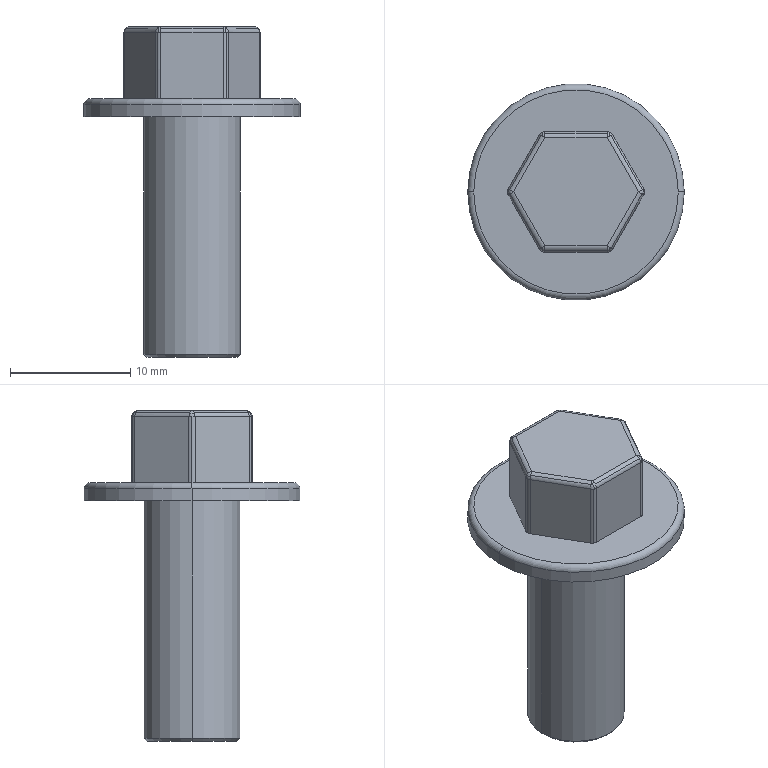Part | SolidWorks | features BaseBody 1 | 1 solid | 54 faces | box 18 x 18 x 27.5 mm | volume 1901 mm3 | cylinder 28 | sphere 12 | plane 10 | cone 2 | torus 2 | commonest cylinder face diameters 1 x24 8 x2 18 x2
STEP:
#1=CARTESIAN_POINT('',(3.75,0.,-20.));
#2=VERTEX_POINT('',#1);
#3=CARTESIAN_POINT('',(-3.75,0.,-20.));
#4=VERTEX_POINT('',#3);
#5=CARTESIAN_POINT('',(0.,0.,-20.));
#6=DIRECTION('',(0.,0.,1.));
#7=DIRECTION('',(1.,0.,0.));
#8=AXIS2_PLACEMENT_3D('',#5,#6,#7);
#9=CIRCLE('',#8,3.75);
#10=EDGE_CURVE('',#2,#4,#9,.T.);
#11=ORIENTED_EDGE('',*,*,#10,.T.);
#12=CARTESIAN_POINT('',(-4.,0.,-19.75));
#13=VERTEX_POINT('',#12);
#14=CARTESIAN_POINT('',(-3.875,0.,-19.875));
#15=DIRECTION('',(-0.7071,0.,0.7071));
#16=VECTOR('',#15,1000.);
#17=LINE('',#14,#16);
#18=EDGE_CURVE('',#4,#13,#17,.T.);
#19=ORIENTED_EDGE('',*,*,#18,.T.);
#20=CARTESIAN_POINT('',(4.,0.,-19.75));
#21=VERTEX_POINT('',#20);
#22=CARTESIAN_POINT('',(0.,0.,-19.75));
#23=DIRECTION('',(0.,0.,-1.));
#24=DIRECTION('',(1.,0.,0.));
#25=AXIS2_PLACEMENT_3D('',#22,#23,#24);
#26=CIRCLE('',#25,4.);
#27=EDGE_CURVE('',#13,#21,#26,.T.);
#28=ORIENTED_EDGE('',*,*,#27,.T.);
#29=CARTESIAN_POINT('',(3.875,0.,-19.875));
#30=DIRECTION('',(0.7071,0.,0.7071));
#31=VECTOR('',#30,1000.);
#32=LINE('',#29,#31);
#33=EDGE_CURVE('',#2,#21,#32,.T.);
#34=ORIENTED_EDGE('',*,*,#33,.F.);
#35=EDGE_LOOP('',(#11,#19,#28,#34));
#36=FACE_OUTER_BOUND('',#35,.T.);
#37=CARTESIAN_POINT('',(0.,0.,-19.875));
#38=DIRECTION('',(0.,0.,1.));
#39=DIRECTION('',(1.,0.,0.));
#40=AXIS2_PLACEMENT_3D('',#37,#38,#39);
#41=CONICAL_SURFACE('',#40,3.875,0.7854);
#42=ADVANCED_FACE('',(#36),#41,.T.);
#43=ORIENTED_EDGE('',*,*,#27,.F.);
#44=CARTESIAN_POINT('',(-4.,0.,0.));
#45=VERTEX_POINT('',#44);
#46=CARTESIAN_POINT('',(-4.,0.,0.));
#47=DIRECTION('',(0.,0.,1.));
#48=VECTOR('',#47,1000.);
#49=LINE('',#46,#48);
#50=EDGE_CURVE('',#13,#45,#49,.T.);
#51=ORIENTED_EDGE('',*,*,#50,.T.);
#52=CARTESIAN_POINT('',(4.,0.,0.));
#53=VERTEX_POINT('',#52);
#54=CARTESIAN_POINT('',(0.,0.,0.));
#55=DIRECTION('',(0.,0.,1.));
#56=DIRECTION('',(1.,0.,0.));
#57=AXIS2_PLACEMENT_3D('',#54,#55,#56);
#58=CIRCLE('',#57,4.);
#59=EDGE_CURVE('',#53,#45,#58,.T.);
#60=ORIENTED_EDGE('',*,*,#59,.F.);
#61=CARTESIAN_POINT('',(4.,0.,0.));
#62=DIRECTION('',(0.,0.,1.));
#63=VECTOR('',#62,1000.);
#64=LINE('',#61,#63);
#65=EDGE_CURVE('',#21,#53,#64,.T.);
#66=ORIENTED_EDGE('',*,*,#65,.F.);
#67=EDGE_LOOP('',(#43,#51,#60,#66));
#68=FACE_OUTER_BOUND('',#67,.T.);
#69=CARTESIAN_POINT('',(0.,0.,0.));
#70=DIRECTION('',(0.,0.,1.));
#71=DIRECTION('',(1.,0.,0.));
#72=AXIS2_PLACEMENT_3D('',#69,#70,#71);
#73=CYLINDRICAL_SURFACE('',#72,4.);
#74=ADVANCED_FACE('',(#68),#73,.T.);
#75=CARTESIAN_POINT('',(-2.784,-4.964,7.));
#76=VERTEX_POINT('',#75);
#77=CARTESIAN_POINT('',(-2.848,-4.933,7.));
#78=VERTEX_POINT('',#77);
#79=CARTESIAN_POINT('',(-2.598,-4.5,7.));
#80=DIRECTION('',(0.,0.,-1.));
#81=DIRECTION('',(0.,-1.,0.));
#82=AXIS2_PLACEMENT_3D('',#79,#80,#81);
#83=CIRCLE('',#82,0.5);
#84=EDGE_CURVE('',#76,#78,#83,.T.);
#85=ORIENTED_EDGE('',*,*,#84,.F.);
#86=CARTESIAN_POINT('',(-2.759,-4.593,7.464));
#87=VERTEX_POINT('',#86);
#88=CARTESIAN_POINT('',(-2.598,-4.5,7.));
#89=DIRECTION('',(-0.9014,0.3603,-0.2402));
#90=DIRECTION('',(-0.3712,-0.9286,0.));
#91=AXIS2_PLACEMENT_3D('',#88,#89,#90);
#92=CIRCLE('',#91,0.5);
#93=EDGE_CURVE('',#76,#87,#92,.T.);
#94=ORIENTED_EDGE('',*,*,#93,.T.);
#95=CARTESIAN_POINT('',(-2.904,-4.677,7.354));
#96=VERTEX_POINT('',#95);
#97=CARTESIAN_POINT('',(-2.598,-4.5,7.));
#98=DIRECTION('',(-0.5,0.866,0.));
#99=DIRECTION('',(-0.866,-0.5,0.));
#100=AXIS2_PLACEMENT_3D('',#97,#98,#99);
#101=CIRCLE('',#100,0.5);
#102=EDGE_CURVE('',#96,#87,#101,.T.);
#103=ORIENTED_EDGE('',*,*,#102,.F.);
#104=CARTESIAN_POINT('',(-3.031,-4.75,7.));
#105=VERTEX_POINT('',#104);
#106=CARTESIAN_POINT('',(-2.598,-4.5,7.));
#107=DIRECTION('',(-0.5,0.866,0.));
#108=DIRECTION('',(-0.866,-0.5,0.));
#109=AXIS2_PLACEMENT_3D('',#106,#107,#108);
#110=CIRCLE('',#109,0.5);
#111=EDGE_CURVE('',#105,#96,#110,.T.);
#112=ORIENTED_EDGE('',*,*,#111,.F.);
#113=CARTESIAN_POINT('',(-2.598,-4.5,7.));
#114=DIRECTION('',(0.,0.,-1.));
#115=DIRECTION('',(0.,-1.,0.));
#116=AXIS2_PLACEMENT_3D('',#113,#114,#115);
#117=CIRCLE('',#116,0.5);
#118=EDGE_CURVE('',#78,#105,#117,.T.);
#119=ORIENTED_EDGE('',*,*,#118,.F.);
#120=EDGE_LOOP('',(#85,#94,#103,#112,#119));
#121=FACE_OUTER_BOUND('',#120,.T.);
#122=CARTESIAN_POINT('',(-2.598,-4.5,7.));
#123=DIRECTION('',(0.9014,-0.3603,0.2402));
#124=DIRECTION('',(-0.433,-0.75,0.5));
#125=AXIS2_PLACEMENT_3D('',#122,#123,#124);
#126=SPHERICAL_SURFACE('',#125,0.5);
#127=ADVANCED_FACE('',(#121),#126,.T.);
#128=CARTESIAN_POINT('',(-2.598,-5.,7.));
#129=VERTEX_POINT('',#128);
#130=CARTESIAN_POINT('',(-2.598,-4.5,7.));
#131=DIRECTION('',(0.,0.,-1.));
#132=DIRECTION('',(0.,-1.,0.));
#133=AXIS2_PLACEMENT_3D('',#130,#131,#132);
#134=CIRCLE('',#133,0.5);
#135=EDGE_CURVE('',#129,#76,#134,.T.);
#136=ORIENTED_EDGE('',*,*,#135,.T.);
#137=ORIENTED_EDGE('',*,*,#84,.T.);
#138=CARTESIAN_POINT('',(-2.848,-4.933,1.5));
#139=VERTEX_POINT('',#138);
#140=CARTESIAN_POINT('',(-2.848,-4.933,1.5));
#141=DIRECTION('',(0.,0.,-1.));
#142=VECTOR('',#141,1000.);
#143=LINE('',#140,#142);
#144=EDGE_CURVE('',#78,#139,#143,.T.);
#145=ORIENTED_EDGE('',*,*,#144,.T.);
#146=CARTESIAN_POINT('',(-2.598,-5.,1.5));
#147=VERTEX_POINT('',#146);
#148=CARTESIAN_POINT('',(-2.598,-4.5,1.5));
#149=DIRECTION('',(0.,0.,1.));
#150=DIRECTION('',(-0.5,-0.866,0.));
#151=AXIS2_PLACEMENT_3D('',#148,#149,#150);
#152=CIRCLE('',#151,0.5);
#153=EDGE_CURVE('',#139,#147,#152,.T.);
#154=ORIENTED_EDGE('',*,*,#153,.T.);
#155=CARTESIAN_POINT('',(-2.598,-5.,1.5));
#156=DIRECTION('',(0.,0.,1.));
#157=VECTOR('',#156,1000.);
#158=LINE('',#155,#157);
#159=EDGE_CURVE('',#147,#129,#158,.T.);
#160=ORIENTED_EDGE('',*,*,#159,.T.);
#161=EDGE_LOOP('',(#136,#137,#145,#154,#160));
#162=FACE_OUTER_BOUND('',#161,.T.);
#163=CARTESIAN_POINT('',(-2.598,-4.5,1.5));
#164=DIRECTION('',(0.,0.,-1.));
#165=DIRECTION('',(-0.5,-0.866,0.));
#166=AXIS2_PLACEMENT_3D('',#163,#164,#165);
#167=CYLINDRICAL_SURFACE('',#166,0.5);
#168=ADVANCED_FACE('',(#162),#167,.T.);
#169=CARTESIAN_POINT('',(2.784,-4.964,7.));
#170=VERTEX_POINT('',#169);
#171=CARTESIAN_POINT('',(2.598,-5.,7.));
#172=VERTEX_POINT('',#171);
#173=CARTESIAN_POINT('',(2.598,-4.5,7.));
#174=DIRECTION('',(0.,0.,-1.));
#175=DIRECTION('',(0.866,-0.5,0.));
#176=AXIS2_PLACEMENT_3D('',#173,#174,#175);
#177=CIRCLE('',#176,0.5);
#178=EDGE_CURVE('',#170,#172,#177,.T.);
#179=ORIENTED_EDGE('',*,*,#178,.F.);
#180=CARTESIAN_POINT('',(2.759,-4.593,7.464));
#181=VERTEX_POINT('',#180);
#182=CARTESIAN_POINT('',(2.598,-4.5,7.));
#183=DIRECTION('',(-0.9014,-0.3603,0.2402));
#184=DIRECTION('',(0.3712,-0.9286,0.));
#185=AXIS2_PLACEMENT_3D('',#182,#183,#184);
#186=CIRCLE('',#185,0.5);
#187=EDGE_CURVE('',#170,#181,#186,.T.);
#188=ORIENTED_EDGE('',*,*,#187,.T.);
#189=CARTESIAN_POINT('',(2.598,-4.5,7.5));
#190=VERTEX_POINT('',#189);
#191=CARTESIAN_POINT('',(2.598,-4.5,7.));
#192=DIRECTION('',(0.5,0.866,0.));
#193=DIRECTION('',(0.,0.,1.));
#194=AXIS2_PLACEMENT_3D('',#191,#192,#193);
#195=CIRCLE('',#194,0.5);
#196=EDGE_CURVE('',#190,#181,#195,.T.);
#197=ORIENTED_EDGE('',*,*,#196,.F.);
#198=CARTESIAN_POINT('',(2.598,-4.854,7.354));
#199=VERTEX_POINT('',#198);
#200=CARTESIAN_POINT('',(2.598,-4.5,7.));
#201=DIRECTION('',(-1.,0.,0.));
#202=DIRECTION('',(0.,-1.,0.));
#203=AXIS2_PLACEMENT_3D('',#200,#201,#202);
#204=CIRCLE('',#203,0.5);
#205=EDGE_CURVE('',#199,#190,#204,.T.);
#206=ORIENTED_EDGE('',*,*,#205,.F.);
#207=CARTESIAN_POINT('',(2.598,-4.5,7.));
#208=DIRECTION('',(-1.,0.,0.));
#209=DIRECTION('',(0.,-1.,0.));
#210=AXIS2_PLACEMENT_3D('',#207,#208,#209);
#211=CIRCLE('',#210,0.5);
#212=EDGE_CURVE('',#172,#199,#211,.T.);
#213=ORIENTED_EDGE('',*,*,#212,.F.);
#214=EDGE_LOOP('',(#179,#188,#197,#206,#213));
#215=FACE_OUTER_BOUND('',#214,.T.);
#216=CARTESIAN_POINT('',(2.598,-4.5,7.));
#217=DIRECTION('',(0.9014,0.3603,-0.2402));
#218=DIRECTION('',(0.433,-0.75,0.5));
#219=AXIS2_PLACEMENT_3D('',#216,#217,#218);
#220=SPHERICAL_SURFACE('',#219,0.5);
#221=ADVANCED_FACE('',(#215),#220,.T.);
#222=CARTESIAN_POINT('',(3.031,-4.75,7.));
#223=VERTEX_POINT('',#222);
#224=CARTESIAN_POINT('',(2.848,-4.933,7.));
#225=VERTEX_POINT('',#224);
#226=CARTESIAN_POINT('',(2.598,-4.5,7.));
#227=DIRECTION('',(0.,0.,-1.));
#228=DIRECTION('',(0.866,-0.5,0.));
#229=AXIS2_PLACEMENT_3D('',#226,#227,#228);
#230=CIRCLE('',#229,0.5);
#231=EDGE_CURVE('',#223,#225,#230,.T.);
#232=ORIENTED_EDGE('',*,*,#231,.T.);
#233=CARTESIAN_POINT('',(2.848,-4.933,1.5));
#234=VERTEX_POINT('',#233);
#235=CARTESIAN_POINT('',(2.848,-4.933,1.5));
#236=DIRECTION('',(0.,0.,-1.));
#237=VECTOR('',#236,1000.);
#238=LINE('',#235,#237);
#239=EDGE_CURVE('',#225,#234,#238,.T.);
#240=ORIENTED_EDGE('',*,*,#239,.T.);
#241=CARTESIAN_POINT('',(3.031,-4.75,1.5));
#242=VERTEX_POINT('',#241);
#243=CARTESIAN_POINT('',(2.598,-4.5,1.5));
#244=DIRECTION('',(0.,0.,1.));
#245=DIRECTION('',(0.5,-0.866,0.));
#246=AXIS2_PLACEMENT_3D('',#243,#244,#245);
#247=CIRCLE('',#246,0.5);
#248=EDGE_CURVE('',#234,#242,#247,.T.);
#249=ORIENTED_EDGE('',*,*,#248,.T.);
#250=CARTESIAN_POINT('',(3.031,-4.75,1.5));
#251=DIRECTION('',(0.,0.,1.));
#252=VECTOR('',#251,1000.);
#253=LINE('',#250,#252);
#254=EDGE_CURVE('',#242,#223,#253,.T.);
#255=ORIENTED_EDGE('',*,*,#254,.T.);
#256=EDGE_LOOP('',(#232,#240,#249,#255));
#257=FACE_OUTER_BOUND('',#256,.T.);
#258=CARTESIAN_POINT('',(2.598,-4.5,1.5));
#259=DIRECTION('',(0.,0.,-1.));
#260=DIRECTION('',(0.5,-0.866,0.));
#261=AXIS2_PLACEMENT_3D('',#258,#259,#260);
#262=CYLINDRICAL_SURFACE('',#261,0.5);
#263=ADVANCED_FACE('',(#257),#262,.T.);
#264=CARTESIAN_POINT('',(-5.583,-0.2236,7.224));
#265=VERTEX_POINT('',#264);
#266=CARTESIAN_POINT('',(-5.629,-0.25,7.));
#267=VERTEX_POINT('',#266);
#268=CARTESIAN_POINT('',(-5.196,0.,7.));
#269=DIRECTION('',(0.5,-0.866,0.));
#270=DIRECTION('',(0.,0.,1.));
#271=AXIS2_PLACEMENT_3D('',#268,#269,#270);
#272=CIRCLE('',#271,0.5);
#273=EDGE_CURVE('',#265,#267,#272,.T.);
#274=ORIENTED_EDGE('',*,*,#273,.F.);
#275=CARTESIAN_POINT('',(-5.583,0.2236,7.224));
#276=VERTEX_POINT('',#275);
#277=CARTESIAN_POINT('',(-5.196,0.,7.));
#278=DIRECTION('',(-0.5,0.,-0.866));
#279=DIRECTION('',(-0.866,0.,0.5));
#280=AXIS2_PLACEMENT_3D('',#277,#278,#279);
#281=CIRCLE('',#280,0.5);
#282=EDGE_CURVE('',#265,#276,#281,.T.);
#283=ORIENTED_EDGE('',*,*,#282,.T.);
#284=CARTESIAN_POINT('',(-5.629,0.25,7.));
#285=VERTEX_POINT('',#284);
#286=CARTESIAN_POINT('',(-5.196,0.,7.));
#287=DIRECTION('',(0.5,0.866,0.));
#288=DIRECTION('',(-0.866,0.5,0.));
#289=AXIS2_PLACEMENT_3D('',#286,#287,#288);
#290=CIRCLE('',#289,0.5);
#291=EDGE_CURVE('',#285,#276,#290,.T.);
#292=ORIENTED_EDGE('',*,*,#291,.F.);
#293=CARTESIAN_POINT('',(-5.696,0.,7.));
#294=VERTEX_POINT('',#293);
#295=CARTESIAN_POINT('',(-5.196,0.,7.));
#296=DIRECTION('',(0.,0.,-1.));
#297=DIRECTION('',(-0.866,-0.5,0.));
#298=AXIS2_PLACEMENT_3D('',#295,#296,#297);
#299=CIRCLE('',#298,0.5);
#300=EDGE_CURVE('',#294,#285,#299,.T.);
#301=ORIENTED_EDGE('',*,*,#300,.F.);
#302=CARTESIAN_POINT('',(-5.196,0.,7.));
#303=DIRECTION('',(0.,0.,-1.));
#304=DIRECTION('',(-0.866,-0.5,0.));
#305=AXIS2_PLACEMENT_3D('',#302,#303,#304);
#306=CIRCLE('',#305,0.5);
#307=EDGE_CURVE('',#267,#294,#306,.T.);
#308=ORIENTED_EDGE('',*,*,#307,.F.);
#309=EDGE_LOOP('',(#274,#283,#292,#301,#308));
#310=FACE_OUTER_BOUND('',#309,.T.);
#311=CARTESIAN_POINT('',(-5.196,0.,7.));
#312=DIRECTION('',(0.5,0.,0.866));
#313=DIRECTION('',(-0.866,0.,0.5));
#314=AXIS2_PLACEMENT_3D('',#311,#312,#313);
#315=SPHERICAL_SURFACE('',#314,0.5);
#316=ADVANCED_FACE('',(#310),#315,.T.);
#317=ORIENTED_EDGE('',*,*,#307,.T.);
#318=CARTESIAN_POINT('',(-5.696,0.,1.5));
#319=VERTEX_POINT('',#318);
#320=CARTESIAN_POINT('',(-5.696,0.,1.5));
#321=DIRECTION('',(0.,0.,-1.));
#322=VECTOR('',#321,1000.);
#323=LINE('',#320,#322);
#324=EDGE_CURVE('',#294,#319,#323,.T.);
#325=ORIENTED_EDGE('',*,*,#324,.T.);
#326=CARTESIAN_POINT('',(-5.629,-0.25,1.5));
#327=VERTEX_POINT('',#326);
#328=CARTESIAN_POINT('',(-5.196,0.,1.5));
#329=DIRECTION('',(0.,0.,1.));
#330=DIRECTION('',(-1.,0.,0.));
#331=AXIS2_PLACEMENT_3D('',#328,#329,#330);
#332=CIRCLE('',#331,0.5);
#333=EDGE_CURVE('',#319,#327,#332,.T.);
#334=ORIENTED_EDGE('',*,*,#333,.T.);
#335=CARTESIAN_POINT('',(-5.629,-0.25,1.5));
#336=DIRECTION('',(0.,0.,1.));
#337=VECTOR('',#336,1000.);
#338=LINE('',#335,#337);
#339=EDGE_CURVE('',#327,#267,#338,.T.);
#340=ORIENTED_EDGE('',*,*,#339,.T.);
#341=EDGE_LOOP('',(#317,#325,#334,#340));
#342=FACE_OUTER_BOUND('',#341,.T.);
#343=CARTESIAN_POINT('',(-5.196,0.,1.5));
#344=DIRECTION('',(0.,0.,-1.));
#345=DIRECTION('',(-1.,0.,0.));
#346=AXIS2_PLACEMENT_3D('',#343,#344,#345);
#347=CYLINDRICAL_SURFACE('',#346,0.5);
#348=ADVANCED_FACE('',(#342),#347,.T.);
#349=ORIENTED_EDGE('',*,*,#111,.T.);
#350=CARTESIAN_POINT('',(-5.502,-0.1768,7.354));
#351=VERTEX_POINT('',#350);
#352=CARTESIAN_POINT('',(-4.925,-1.177,7.354));
#353=DIRECTION('',(-0.5,0.866,0.));
#354=VECTOR('',#353,1000.);
#355=LINE('',#352,#354);
#356=EDGE_CURVE('',#96,#351,#355,.T.);
#357=ORIENTED_EDGE('',*,*,#356,.T.);
#358=CARTESIAN_POINT('',(-5.196,0.,7.));
#359=DIRECTION('',(0.5,-0.866,0.));
#360=DIRECTION('',(0.,0.,1.));
#361=AXIS2_PLACEMENT_3D('',#358,#359,#360);
#362=CIRCLE('',#361,0.5);
#363=EDGE_CURVE('',#351,#265,#362,.T.);
#364=ORIENTED_EDGE('',*,*,#363,.T.);
#365=ORIENTED_EDGE('',*,*,#273,.T.);
#366=CARTESIAN_POINT('',(-5.052,-1.25,7.));
#367=DIRECTION('',(0.5,-0.866,0.));
#368=VECTOR('',#367,1000.);
#369=LINE('',#366,#368);
#370=EDGE_CURVE('',#267,#105,#369,.T.);
#371=ORIENTED_EDGE('',*,*,#370,.T.);
#372=EDGE_LOOP('',(#349,#357,#364,#365,#371));
#373=FACE_OUTER_BOUND('',#372,.T.);
#374=CARTESIAN_POINT('',(-4.619,-1.,7.));
#375=DIRECTION('',(-0.5,0.866,0.));
#376=DIRECTION('',(-0.6124,-0.3536,0.7071));
#377=AXIS2_PLACEMENT_3D('',#374,#375,#376);
#378=CYLINDRICAL_SURFACE('',#377,0.5);
#379=ADVANCED_FACE('',(#373),#378,.T.);
#380=CARTESIAN_POINT('',(5.583,0.2236,7.224));
#381=VERTEX_POINT('',#380);
#382=CARTESIAN_POINT('',(5.629,0.25,7.));
#383=VERTEX_POINT('',#382);
#384=CARTESIAN_POINT('',(5.196,0.,7.));
#385=DIRECTION('',(-0.5,0.866,0.));
#386=DIRECTION('',(0.,0.,1.));
#387=AXIS2_PLACEMENT_3D('',#384,#385,#386);
#388=CIRCLE('',#387,0.5);
#389=EDGE_CURVE('',#381,#383,#388,.T.);
#390=ORIENTED_EDGE('',*,*,#389,.F.);
#391=CARTESIAN_POINT('',(5.583,-0.2236,7.224));
#392=VERTEX_POINT('',#391);
#393=CARTESIAN_POINT('',(5.196,0.,7.));
#394=DIRECTION('',(0.5,0.,-0.866));
#395=DIRECTION('',(-0.866,0.,-0.5));
#396=AXIS2_PLACEMENT_3D('',#393,#394,#395);
#397=CIRCLE('',#396,0.5);
#398=EDGE_CURVE('',#381,#392,#397,.T.);
#399=ORIENTED_EDGE('',*,*,#398,.T.);
#400=CARTESIAN_POINT('',(5.629,-0.25,7.));
#401=VERTEX_POINT('',#400);
#402=CARTESIAN_POINT('',(5.196,0.,7.));
#403=DIRECTION('',(-0.5,-0.866,0.));
#404=DIRECTION('',(0.866,-0.5,0.));
#405=AXIS2_PLACEMENT_3D('',#402,#403,#404);
#406=CIRCLE('',#405,0.5);
#407=EDGE_CURVE('',#401,#392,#406,.T.);
#408=ORIENTED_EDGE('',*,*,#407,.F.);
#409=CARTESIAN_POINT('',(5.696,0.,7.));
#410=VERTEX_POINT('',#409);
#411=CARTESIAN_POINT('',(5.196,0.,7.));
#412=DIRECTION('',(0.,0.,-1.));
#413=DIRECTION('',(0.866,0.5,0.));
#414=AXIS2_PLACEMENT_3D('',#411,#412,#413);
#415=CIRCLE('',#414,0.5);
#416=EDGE_CURVE('',#410,#401,#415,.T.);
#417=ORIENTED_EDGE('',*,*,#416,.F.);
#418=CARTESIAN_POINT('',(5.196,0.,7.));
#419=DIRECTION('',(0.,0.,-1.));
#420=DIRECTION('',(0.866,0.5,0.));
#421=AXIS2_PLACEMENT_3D('',#418,#419,#420);
#422=CIRCLE('',#421,0.5);
#423=EDGE_CURVE('',#383,#410,#422,.T.);
#424=ORIENTED_EDGE('',*,*,#423,.F.);
#425=EDGE_LOOP('',(#390,#399,#408,#417,#424));
#426=FACE_OUTER_BOUND('',#425,.T.);
#427=CARTESIAN_POINT('',(5.196,0.,7.));
#428=DIRECTION('',(-0.5,0.,0.866));
#429=DIRECTION('',(0.866,0.,0.5));
#430=AXIS2_PLACEMENT_3D('',#427,#428,#429);
#431=SPHERICAL_SURFACE('',#430,0.5);
#432=ADVANCED_FACE('',(#426),#431,.T.);
#433=ORIENTED_EDGE('',*,*,#423,.T.);
#434=CARTESIAN_POINT('',(5.696,0.,1.5));
#435=VERTEX_POINT('',#434);
#436=CARTESIAN_POINT('',(5.696,0.,1.5));
#437=DIRECTION('',(0.,0.,-1.));
#438=VECTOR('',#437,1000.);
#439=LINE('',#436,#438);
#440=EDGE_CURVE('',#410,#435,#439,.T.);
#441=ORIENTED_EDGE('',*,*,#440,.T.);
#442=CARTESIAN_POINT('',(5.629,0.25,1.5));
#443=VERTEX_POINT('',#442);
#444=CARTESIAN_POINT('',(5.196,0.,1.5));
#445=DIRECTION('',(0.,0.,1.));
#446=DIRECTION('',(1.,0.,0.));
#447=AXIS2_PLACEMENT_3D('',#444,#445,#446);
#448=CIRCLE('',#447,0.5);
#449=EDGE_CURVE('',#435,#443,#448,.T.);
#450=ORIENTED_EDGE('',*,*,#449,.T.);
#451=CARTESIAN_POINT('',(5.629,0.25,1.5));
#452=DIRECTION('',(0.,0.,1.));
#453=VECTOR('',#452,1000.);
#454=LINE('',#451,#453);
#455=EDGE_CURVE('',#443,#383,#454,.T.);
#456=ORIENTED_EDGE('',*,*,#455,.T.);
#457=EDGE_LOOP('',(#433,#441,#450,#456));
#458=FACE_OUTER_BOUND('',#457,.T.);
#459=CARTESIAN_POINT('',(5.196,0.,1.5));
#460=DIRECTION('',(0.,0.,-1.));
#461=DIRECTION('',(1.,0.,0.));
#462=AXIS2_PLACEMENT_3D('',#459,#460,#461);
#463=CYLINDRICAL_SURFACE('',#462,0.5);
#464=ADVANCED_FACE('',(#458),#463,.T.);
#465=CARTESIAN_POINT('',(-2.759,4.593,7.464));
#466=VERTEX_POINT('',#465);
#467=CARTESIAN_POINT('',(-2.904,4.677,7.354));
#468=VERTEX_POINT('',#467);
#469=CARTESIAN_POINT('',(-2.598,4.5,7.));
#470=DIRECTION('',(-0.5,-0.866,0.));
#471=DIRECTION('',(0.,0.,1.));
#472=AXIS2_PLACEMENT_3D('',#469,#470,#471);
#473=CIRCLE('',#472,0.5);
#474=EDGE_CURVE('',#466,#468,#473,.T.);
#475=ORIENTED_EDGE('',*,*,#474,.F.);
#476=CARTESIAN_POINT('',(-2.784,4.964,7.));
#477=VERTEX_POINT('',#476);
#478=CARTESIAN_POINT('',(-2.598,4.5,7.));
#479=DIRECTION('',(-0.9014,-0.3603,-0.2402));
#480=DIRECTION('',(0.3712,-0.9286,0.));
#481=AXIS2_PLACEMENT_3D('',#478,#479,#480);
#482=CIRCLE('',#481,0.5);
#483=EDGE_CURVE('',#466,#477,#482,.T.);
#484=ORIENTED_EDGE('',*,*,#483,.T.);
#485=CARTESIAN_POINT('',(-2.848,4.933,7.));
#486=VERTEX_POINT('',#485);
#487=CARTESIAN_POINT('',(-2.598,4.5,7.));
#488=DIRECTION('',(0.,0.,-1.));
#489=DIRECTION('',(-0.866,0.5,0.));
#490=AXIS2_PLACEMENT_3D('',#487,#488,#489);
#491=CIRCLE('',#490,0.5);
#492=EDGE_CURVE('',#486,#477,#491,.T.);
#493=ORIENTED_EDGE('',*,*,#492,.F.);
#494=CARTESIAN_POINT('',(-3.031,4.75,7.));
#495=VERTEX_POINT('',#494);
#496=CARTESIAN_POINT('',(-2.598,4.5,7.));
#497=DIRECTION('',(0.,0.,-1.));
#498=DIRECTION('',(-0.866,0.5,0.));
#499=AXIS2_PLACEMENT_3D('',#496,#497,#498);
#500=CIRCLE('',#499,0.5);
#501=EDGE_CURVE('',#495,#486,#500,.T.);
#502=ORIENTED_EDGE('',*,*,#501,.F.);
#503=CARTESIAN_POINT('',(-2.598,4.5,7.));
#504=DIRECTION('',(-0.5,-0.866,0.));
#505=DIRECTION('',(0.,0.,1.));
#506=AXIS2_PLACEMENT_3D('',#503,#504,#505);
#507=CIRCLE('',#506,0.5);
#508=EDGE_CURVE('',#468,#495,#507,.T.);
#509=ORIENTED_EDGE('',*,*,#508,.F.);
#510=EDGE_LOOP('',(#475,#484,#493,#502,#509));
#511=FACE_OUTER_BOUND('',#510,.T.);
#512=CARTESIAN_POINT('',(-2.598,4.5,7.));
#513=DIRECTION('',(0.9014,0.3603,0.2402));
#514=DIRECTION('',(-0.433,0.75,0.5));
#515=AXIS2_PLACEMENT_3D('',#512,#513,#514);
#516=SPHERICAL_SURFACE('',#515,0.5);
#517=ADVANCED_FACE('',(#511),#516,.T.);
#518=ORIENTED_EDGE('',*,*,#501,.T.);
#519=CARTESIAN_POINT('',(-2.848,4.933,1.5));
#520=VERTEX_POINT('',#519);
#521=CARTESIAN_POINT('',(-2.848,4.933,1.5));
#522=DIRECTION('',(0.,0.,-1.));
#523=VECTOR('',#522,1000.);
#524=LINE('',#521,#523);
#525=EDGE_CURVE('',#486,#520,#524,.T.);
#526=ORIENTED_EDGE('',*,*,#525,.T.);
#527=CARTESIAN_POINT('',(-3.031,4.75,1.5));
#528=VERTEX_POINT('',#527);
#529=CARTESIAN_POINT('',(-2.598,4.5,1.5));
#530=DIRECTION('',(0.,0.,1.));
#531=DIRECTION('',(-0.5,0.866,0.));
#532=AXIS2_PLACEMENT_3D('',#529,#530,#531);
#533=CIRCLE('',#532,0.5);
#534=EDGE_CURVE('',#520,#528,#533,.T.);
#535=ORIENTED_EDGE('',*,*,#534,.T.);
#536=CARTESIAN_POINT('',(-3.031,4.75,1.5));
#537=DIRECTION('',(0.,0.,1.));
#538=VECTOR('',#537,1000.);
#539=LINE('',#536,#538);
#540=EDGE_CURVE('',#528,#495,#539,.T.);
#541=ORIENTED_EDGE('',*,*,#540,.T.);
#542=EDGE_LOOP('',(#518,#526,#535,#541));
#543=FACE_OUTER_BOUND('',#542,.T.);
#544=CARTESIAN_POINT('',(-2.598,4.5,1.5));
#545=DIRECTION('',(0.,0.,-1.));
#546=DIRECTION('',(-0.5,0.866,0.));
#547=AXIS2_PLACEMENT_3D('',#544,#545,#546);
#548=CYLINDRICAL_SURFACE('',#547,0.5);
#549=ADVANCED_FACE('',(#543),#548,.T.);
#550=ORIENTED_EDGE('',*,*,#291,.T.);
#551=CARTESIAN_POINT('',(-5.502,0.1768,7.354));
#552=VERTEX_POINT('',#551);
#553=CARTESIAN_POINT('',(-5.196,0.,7.));
#554=DIRECTION('',(0.5,0.866,0.));
#555=DIRECTION('',(-0.866,0.5,0.));
#556=AXIS2_PLACEMENT_3D('',#553,#554,#555);
#557=CIRCLE('',#556,0.5);
#558=EDGE_CURVE('',#276,#552,#557,.T.);
#559=ORIENTED_EDGE('',*,*,#558,.T.);
#560=CARTESIAN_POINT('',(-3.482,3.677,7.354));
#561=DIRECTION('',(0.5,0.866,0.));
#562=VECTOR('',#561,1000.);
#563=LINE('',#560,#562);
#564=EDGE_CURVE('',#552,#468,#563,.T.);
#565=ORIENTED_EDGE('',*,*,#564,.T.);
#566=ORIENTED_EDGE('',*,*,#508,.T.);
#567=CARTESIAN_POINT('',(-3.608,3.75,7.));
#568=DIRECTION('',(-0.5,-0.866,0.));
#569=VECTOR('',#568,1000.);
#570=LINE('',#567,#569);
#571=EDGE_CURVE('',#495,#285,#570,.T.);
#572=ORIENTED_EDGE('',*,*,#571,.T.);
#573=EDGE_LOOP('',(#550,#559,#565,#566,#572));
#574=FACE_OUTER_BOUND('',#573,.T.);
#575=CARTESIAN_POINT('',(-3.175,3.5,7.));
#576=DIRECTION('',(0.5,0.866,0.));
#577=DIRECTION('',(-0.6124,0.3536,0.7071));
#578=AXIS2_PLACEMENT_3D('',#575,#576,#577);
#579=CYLINDRICAL_SURFACE('',#578,0.5);
#580=ADVANCED_FACE('',(#574),#579,.T.);
#581=CARTESIAN_POINT('',(2.759,4.593,7.464));
#582=VERTEX_POINT('',#581);
#583=CARTESIAN_POINT('',(2.598,4.5,7.5));
#584=VERTEX_POINT('',#583);
#585=CARTESIAN_POINT('',(2.598,4.5,7.));
#586=DIRECTION('',(0.5,-0.866,0.));
#587=DIRECTION('',(0.866,0.5,0.));
#588=AXIS2_PLACEMENT_3D('',#585,#586,#587);
#589=CIRCLE('',#588,0.5);
#590=EDGE_CURVE('',#582,#584,#589,.T.);
#591=ORIENTED_EDGE('',*,*,#590,.F.);
#592=CARTESIAN_POINT('',(2.784,4.964,7.));
#593=VERTEX_POINT('',#592);
#594=CARTESIAN_POINT('',(2.598,4.5,7.));
#595=DIRECTION('',(-0.9014,0.3603,0.2402));
#596=DIRECTION('',(-0.3712,-0.9286,0.));
#597=AXIS2_PLACEMENT_3D('',#594,#595,#596);
#598=CIRCLE('',#597,0.5);
#599=EDGE_CURVE('',#582,#593,#598,.T.);
#600=ORIENTED_EDGE('',*,*,#599,.T.);
#601=CARTESIAN_POINT('',(2.598,5.,7.));
#602=VERTEX_POINT('',#601);
#603=CARTESIAN_POINT('',(2.598,4.5,7.));
#604=DIRECTION('',(0.,0.,-1.));
#605=DIRECTION('',(0.,1.,0.));
#606=AXIS2_PLACEMENT_3D('',#603,#604,#605);
#607=CIRCLE('',#606,0.5);
#608=EDGE_CURVE('',#602,#593,#607,.T.);
#609=ORIENTED_EDGE('',*,*,#608,.F.);
#610=CARTESIAN_POINT('',(2.598,4.854,7.354));
#611=VERTEX_POINT('',#610);
#612=CARTESIAN_POINT('',(2.598,4.5,7.));
#613=DIRECTION('',(-1.,0.,0.));
#614=DIRECTION('',(0.,0.,1.));
#615=AXIS2_PLACEMENT_3D('',#612,#613,#614);
#616=CIRCLE('',#615,0.5);
#617=EDGE_CURVE('',#611,#602,#616,.T.);
#618=ORIENTED_EDGE('',*,*,#617,.F.);
#619=CARTESIAN_POINT('',(2.598,4.5,7.));
#620=DIRECTION('',(-1.,0.,0.));
#621=DIRECTION('',(0.,0.,1.));
#622=AXIS2_PLACEMENT_3D('',#619,#620,#621);
#623=CIRCLE('',#622,0.5);
#624=EDGE_CURVE('',#584,#611,#623,.T.);
#625=ORIENTED_EDGE('',*,*,#624,.F.);
#626=EDGE_LOOP('',(#591,#600,#609,#618,#625));
#627=FACE_OUTER_BOUND('',#626,.T.);
#628=CARTESIAN_POINT('',(2.598,4.5,7.));
#629=DIRECTION('',(0.9014,-0.3603,-0.2402));
#630=DIRECTION('',(0.433,0.75,0.5));
#631=AXIS2_PLACEMENT_3D('',#628,#629,#630);
#632=SPHERICAL_SURFACE('',#631,0.5);
#633=ADVANCED_FACE('',(#627),#632,.T.);
#634=ORIENTED_EDGE('',*,*,#608,.T.);
#635=CARTESIAN_POINT('',(2.848,4.933,7.));
#636=VERTEX_POINT('',#635);
#637=CARTESIAN_POINT('',(2.598,4.5,7.));
#638=DIRECTION('',(0.,0.,-1.));
#639=DIRECTION('',(0.,1.,0.));
#640=AXIS2_PLACEMENT_3D('',#637,#638,#639);
#641=CIRCLE('',#640,0.5);
#642=EDGE_CURVE('',#593,#636,#641,.T.);
#643=ORIENTED_EDGE('',*,*,#642,.T.);
#644=CARTESIAN_POINT('',(2.848,4.933,1.5));
#645=VERTEX_POINT('',#644);
#646=CARTESIAN_POINT('',(2.848,4.933,1.5));
#647=DIRECTION('',(0.,0.,-1.));
#648=VECTOR('',#647,1000.);
#649=LINE('',#646,#648);
#650=EDGE_CURVE('',#636,#645,#649,.T.);
#651=ORIENTED_EDGE('',*,*,#650,.T.);
#652=CARTESIAN_POINT('',(2.598,5.,1.5));
#653=VERTEX_POINT('',#652);
#654=CARTESIAN_POINT('',(2.598,4.5,1.5));
#655=DIRECTION('',(0.,0.,1.));
#656=DIRECTION('',(0.5,0.866,0.));
#657=AXIS2_PLACEMENT_3D('',#654,#655,#656);
#658=CIRCLE('',#657,0.5);
#659=EDGE_CURVE('',#645,#653,#658,.T.);
#660=ORIENTED_EDGE('',*,*,#659,.T.);
#661=CARTESIAN_POINT('',(2.598,5.,1.5));
#662=DIRECTION('',(0.,0.,1.));
#663=VECTOR('',#662,1000.);
#664=LINE('',#661,#663);
#665=EDGE_CURVE('',#653,#602,#664,.T.);
#666=ORIENTED_EDGE('',*,*,#665,.T.);
#667=EDGE_LOOP('',(#634,#643,#651,#660,#666));
#668=FACE_OUTER_BOUND('',#667,.T.);
#669=CARTESIAN_POINT('',(2.598,4.5,1.5));
#670=DIRECTION('',(0.,0.,-1.));
#671=DIRECTION('',(0.5,0.866,0.));
#672=AXIS2_PLACEMENT_3D('',#669,#670,#671);
#673=CYLINDRICAL_SURFACE('',#672,0.5);
#674=ADVANCED_FACE('',(#668),#673,.T.);
#675=CARTESIAN_POINT('',(-2.598,5.,7.));
#676=VERTEX_POINT('',#675);
#677=CARTESIAN_POINT('',(-2.598,4.854,7.354));
#678=VERTEX_POINT('',#677);
#679=CARTESIAN_POINT('',(-2.598,4.5,7.));
#680=DIRECTION('',(1.,0.,0.));
#681=DIRECTION('',(0.,1.,0.));
#682=AXIS2_PLACEMENT_3D('',#679,#680,#681);
#683=CIRCLE('',#682,0.5);
#684=EDGE_CURVE('',#676,#678,#683,.T.);
#685=ORIENTED_EDGE('',*,*,#684,.T.);
#686=CARTESIAN_POINT('',(1.443,4.854,7.354));
#687=DIRECTION('',(1.,0.,0.));
#688=VECTOR('',#687,1000.);
#689=LINE('',#686,#688);
#690=EDGE_CURVE('',#678,#611,#689,.T.);
#691=ORIENTED_EDGE('',*,*,#690,.T.);
#692=ORIENTED_EDGE('',*,*,#617,.T.);
#693=CARTESIAN_POINT('',(1.443,5.,7.));
#694=DIRECTION('',(-1.,0.,0.));
#695=VECTOR('',#694,1000.);
#696=LINE('',#693,#695);
#697=EDGE_CURVE('',#602,#676,#696,.T.);
#698=ORIENTED_EDGE('',*,*,#697,.T.);
#699=EDGE_LOOP('',(#685,#691,#692,#698));
#700=FACE_OUTER_BOUND('',#699,.T.);
#701=CARTESIAN_POINT('',(1.443,4.5,7.));
#702=DIRECTION('',(1.,0.,0.));
#703=DIRECTION('',(0.,0.7071,0.7071));
#704=AXIS2_PLACEMENT_3D('',#701,#702,#703);
#705=CYLINDRICAL_SURFACE('',#704,0.5);
#706=ADVANCED_FACE('',(#700),#705,.T.);
#707=CARTESIAN_POINT('',(3.031,4.75,7.));
#708=VERTEX_POINT('',#707);
#709=CARTESIAN_POINT('',(2.904,4.677,7.354));
#710=VERTEX_POINT('',#709);
#711=CARTESIAN_POINT('',(2.598,4.5,7.));
#712=DIRECTION('',(0.5,-0.866,0.));
#713=DIRECTION('',(0.866,0.5,0.));
#714=AXIS2_PLACEMENT_3D('',#711,#712,#713);
#715=CIRCLE('',#714,0.5);
#716=EDGE_CURVE('',#708,#710,#715,.T.);
#717=ORIENTED_EDGE('',*,*,#716,.T.);
#718=CARTESIAN_POINT('',(5.502,0.1768,7.354));
#719=VERTEX_POINT('',#718);
#720=CARTESIAN_POINT('',(4.925,1.177,7.354));
#721=DIRECTION('',(0.5,-0.866,0.));
#722=VECTOR('',#721,1000.);
#723=LINE('',#720,#722);
#724=EDGE_CURVE('',#710,#719,#723,.T.);
#725=ORIENTED_EDGE('',*,*,#724,.T.);
#726=CARTESIAN_POINT('',(5.196,0.,7.));
#727=DIRECTION('',(-0.5,0.866,0.));
#728=DIRECTION('',(0.,0.,1.));
#729=AXIS2_PLACEMENT_3D('',#726,#727,#728);
#730=CIRCLE('',#729,0.5);
#731=EDGE_CURVE('',#719,#381,#730,.T.);
#732=ORIENTED_EDGE('',*,*,#731,.T.);
#733=ORIENTED_EDGE('',*,*,#389,.T.);
#734=CARTESIAN_POINT('',(5.052,1.25,7.));
#735=DIRECTION('',(-0.5,0.866,0.));
#736=VECTOR('',#735,1000.);
#737=LINE('',#734,#736);
#738=EDGE_CURVE('',#383,#708,#737,.T.);
#739=ORIENTED_EDGE('',*,*,#738,.T.);
#740=EDGE_LOOP('',(#717,#725,#732,#733,#739));
#741=FACE_OUTER_BOUND('',#740,.T.);
#742=CARTESIAN_POINT('',(4.619,1.,7.));
#743=DIRECTION('',(0.5,-0.866,0.));
#744=DIRECTION('',(0.6124,0.3536,0.7071));
#745=AXIS2_PLACEMENT_3D('',#742,#743,#744);
#746=CYLINDRICAL_SURFACE('',#745,0.5);
#747=ADVANCED_FACE('',(#741),#746,.T.);
#748=ORIENTED_EDGE('',*,*,#407,.T.);
#749=CARTESIAN_POINT('',(5.502,-0.1768,7.354));
#750=VERTEX_POINT('',#749);
#751=CARTESIAN_POINT('',(5.196,0.,7.));
#752=DIRECTION('',(-0.5,-0.866,0.));
#753=DIRECTION('',(0.866,-0.5,0.));
#754=AXIS2_PLACEMENT_3D('',#751,#752,#753);
#755=CIRCLE('',#754,0.5);
#756=EDGE_CURVE('',#392,#750,#755,.T.);
#757=ORIENTED_EDGE('',*,*,#756,.T.);
#758=CARTESIAN_POINT('',(2.904,-4.677,7.354));
#759=VERTEX_POINT('',#758);
#760=CARTESIAN_POINT('',(3.482,-3.677,7.354));
#761=DIRECTION('',(-0.5,-0.866,0.));
#762=VECTOR('',#761,1000.);
#763=LINE('',#760,#762);
#764=EDGE_CURVE('',#750,#759,#763,.T.);
#765=ORIENTED_EDGE('',*,*,#764,.T.);
#766=CARTESIAN_POINT('',(2.598,-4.5,7.));
#767=DIRECTION('',(0.5,0.866,0.));
#768=DIRECTION('',(0.,0.,1.));
#769=AXIS2_PLACEMENT_3D('',#766,#767,#768);
#770=CIRCLE('',#769,0.5);
#771=EDGE_CURVE('',#759,#223,#770,.T.);
#772=ORIENTED_EDGE('',*,*,#771,.T.);
#773=CARTESIAN_POINT('',(3.608,-3.75,7.));
#774=DIRECTION('',(0.5,0.866,0.));
#775=VECTOR('',#774,1000.);
#776=LINE('',#773,#775);
#777=EDGE_CURVE('',#223,#401,#776,.T.);
#778=ORIENTED_EDGE('',*,*,#777,.T.);
#779=EDGE_LOOP('',(#748,#757,#765,#772,#778));
#780=FACE_OUTER_BOUND('',#779,.T.);
#781=CARTESIAN_POINT('',(3.175,-3.5,7.));
#782=DIRECTION('',(-0.5,-0.866,0.));
#783=DIRECTION('',(0.6124,-0.3536,0.7071));
#784=AXIS2_PLACEMENT_3D('',#781,#782,#783);
#785=CYLINDRICAL_SURFACE('',#784,0.5);
#786=ADVANCED_FACE('',(#780),#785,.T.);
#787=ORIENTED_EDGE('',*,*,#212,.T.);
#788=CARTESIAN_POINT('',(-2.598,-4.854,7.354));
#789=VERTEX_POINT('',#788);
#790=CARTESIAN_POINT('',(-1.443,-4.854,7.354));
#791=DIRECTION('',(-1.,0.,0.));
#792=VECTOR('',#791,1000.);
#793=LINE('',#790,#792);
#794=EDGE_CURVE('',#199,#789,#793,.T.);
#795=ORIENTED_EDGE('',*,*,#794,.T.);
#796=CARTESIAN_POINT('',(-2.598,-4.5,7.));
#797=DIRECTION('',(1.,0.,0.));
#798=DIRECTION('',(0.,0.,1.));
#799=AXIS2_PLACEMENT_3D('',#796,#797,#798);
#800=CIRCLE('',#799,0.5);
#801=EDGE_CURVE('',#789,#129,#800,.T.);
#802=ORIENTED_EDGE('',*,*,#801,.T.);
#803=CARTESIAN_POINT('',(-1.443,-5.,7.));
#804=DIRECTION('',(1.,0.,0.));
#805=VECTOR('',#804,1000.);
#806=LINE('',#803,#805);
#807=EDGE_CURVE('',#129,#172,#806,.T.);
#808=ORIENTED_EDGE('',*,*,#807,.T.);
#809=EDGE_LOOP('',(#787,#795,#802,#808));
#810=FACE_OUTER_BOUND('',#809,.T.);
#811=CARTESIAN_POINT('',(-1.443,-4.5,7.));
#812=DIRECTION('',(-1.,0.,0.));
#813=DIRECTION('',(0.,-0.7071,0.7071));
#814=AXIS2_PLACEMENT_3D('',#811,#812,#813);
#815=CYLINDRICAL_SURFACE('',#814,0.5);
#816=ADVANCED_FACE('',(#810),#815,.T.);
#817=CARTESIAN_POINT('',(9.,0.,1.));
#818=VERTEX_POINT('',#817);
#819=CARTESIAN_POINT('',(-9.,0.,1.));
#820=VERTEX_POINT('',#819);
#821=CARTESIAN_POINT('',(0.,0.,1.));
#822=DIRECTION('',(0.,0.,1.));
#823=DIRECTION('',(-1.,0.,0.));
#824=AXIS2_PLACEMENT_3D('',#821,#822,#823);
#825=CIRCLE('',#824,9.);
#826=EDGE_CURVE('',#818,#820,#825,.T.);
#827=ORIENTED_EDGE('',*,*,#826,.T.);
#828=CARTESIAN_POINT('',(-8.5,0.,1.5));
#829=VERTEX_POINT('',#828);
#830=CARTESIAN_POINT('',(-8.5,0.,1.));
#831=DIRECTION('',(0.,1.,0.));
#832=DIRECTION('',(-1.,0.,0.));
#833=AXIS2_PLACEMENT_3D('',#830,#831,#832);
#834=CIRCLE('',#833,0.5);
#835=EDGE_CURVE('',#820,#829,#834,.T.);
#836=ORIENTED_EDGE('',*,*,#835,.T.);
#837=CARTESIAN_POINT('',(8.5,0.,1.5));
#838=VERTEX_POINT('',#837);
#839=CARTESIAN_POINT('',(0.,0.,1.5));
#840=DIRECTION('',(0.,0.,-1.));
#841=DIRECTION('',(-1.,0.,0.));
#842=AXIS2_PLACEMENT_3D('',#839,#840,#841);
#843=CIRCLE('',#842,8.5);
#844=EDGE_CURVE('',#829,#838,#843,.T.);
#845=ORIENTED_EDGE('',*,*,#844,.T.);
#846=CARTESIAN_POINT('',(8.5,0.,1.));
#847=DIRECTION('',(0.,-1.,0.));
#848=DIRECTION('',(0.,0.,-1.));
#849=AXIS2_PLACEMENT_3D('',#846,#847,#848);
#850=CIRCLE('',#849,0.5);
#851=EDGE_CURVE('',#818,#838,#850,.T.);
#852=ORIENTED_EDGE('',*,*,#851,.F.);
#853=EDGE_LOOP('',(#827,#836,#845,#852));
#854=FACE_OUTER_BOUND('',#853,.T.);
#855=CARTESIAN_POINT('',(0.,0.,1.));
#856=DIRECTION('',(0.,0.,1.));
#857=DIRECTION('',(1.,0.,0.));
#858=AXIS2_PLACEMENT_3D('',#855,#856,#857);
#859=TOROIDAL_SURFACE('',#858,8.5,0.5);
#860=ADVANCED_FACE('',(#854),#859,.T.);
#861=ORIENTED_EDGE('',*,*,#826,.F.);
#862=CARTESIAN_POINT('',(9.,0.,0.));
#863=VERTEX_POINT('',#862);
#864=CARTESIAN_POINT('',(9.,0.,0.));
#865=DIRECTION('',(0.,0.,-1.));
#866=VECTOR('',#865,1000.);
#867=LINE('',#864,#866);
#868=EDGE_CURVE('',#818,#863,#867,.T.);
#869=ORIENTED_EDGE('',*,*,#868,.T.);
#870=CARTESIAN_POINT('',(-9.,0.,0.));
#871=VERTEX_POINT('',#870);
#872=CARTESIAN_POINT('',(0.,0.,0.));
#873=DIRECTION('',(0.,0.,-1.));
#874=DIRECTION('',(-1.,0.,0.));
#875=AXIS2_PLACEMENT_3D('',#872,#873,#874);
#876=CIRCLE('',#875,9.);
#877=EDGE_CURVE('',#871,#863,#876,.T.);
#878=ORIENTED_EDGE('',*,*,#877,.F.);
#879=CARTESIAN_POINT('',(-9.,0.,0.));
#880=DIRECTION('',(0.,0.,-1.));
#881=VECTOR('',#880,1000.);
#882=LINE('',#879,#881);
#883=EDGE_CURVE('',#820,#871,#882,.T.);
#884=ORIENTED_EDGE('',*,*,#883,.F.);
#885=EDGE_LOOP('',(#861,#869,#878,#884));
#886=FACE_OUTER_BOUND('',#885,.T.);
#887=CARTESIAN_POINT('',(0.,0.,0.));
#888=DIRECTION('',(0.,0.,-1.));
#889=DIRECTION('',(-1.,0.,0.));
#890=AXIS2_PLACEMENT_3D('',#887,#888,#889);
#891=CYLINDRICAL_SURFACE('',#890,9.);
#892=ADVANCED_FACE('',(#886),#891,.T.);
#893=ORIENTED_EDGE('',*,*,#10,.F.);
#894=CARTESIAN_POINT('',(0.,0.,-20.));
#895=DIRECTION('',(0.,0.,1.));
#896=DIRECTION('',(1.,0.,0.));
#897=AXIS2_PLACEMENT_3D('',#894,#895,#896);
#898=CIRCLE('',#897,3.75);
#899=EDGE_CURVE('',#4,#2,#898,.T.);
#900=ORIENTED_EDGE('',*,*,#899,.F.);
#901=EDGE_LOOP('',(#893,#900));
#902=FACE_OUTER_BOUND('',#901,.T.);
#903=CARTESIAN_POINT('',(0.,0.,-20.));
#904=DIRECTION('',(0.,0.,1.));
#905=DIRECTION('',(1.,0.,0.));
#906=AXIS2_PLACEMENT_3D('',#903,#904,#905);
#907=PLANE('',#906);
#908=ADVANCED_FACE('',(#902),#907,.F.);
#909=CARTESIAN_POINT('',(-3.031,-4.75,1.5));
#910=VERTEX_POINT('',#909);
#911=CARTESIAN_POINT('',(-3.031,-4.75,1.5));
#912=DIRECTION('',(0.,0.,-1.));
#913=VECTOR('',#912,1000.);
#914=LINE('',#911,#913);
#915=EDGE_CURVE('',#105,#910,#914,.T.);
#916=ORIENTED_EDGE('',*,*,#915,.F.);
#917=ORIENTED_EDGE('',*,*,#370,.F.);
#918=ORIENTED_EDGE('',*,*,#339,.F.);
#919=CARTESIAN_POINT('',(-5.052,-1.25,1.5));
#920=DIRECTION('',(-0.5,0.866,0.));
#921=VECTOR('',#920,1000.);
#922=LINE('',#919,#921);
#923=EDGE_CURVE('',#910,#327,#922,.T.);
#924=ORIENTED_EDGE('',*,*,#923,.F.);
#925=EDGE_LOOP('',(#916,#917,#918,#924));
#926=FACE_OUTER_BOUND('',#925,.T.);
#927=CARTESIAN_POINT('',(-5.774,0.,1.5));
#928=DIRECTION('',(-0.866,-0.5,0.));
#929=DIRECTION('',(-0.5,0.866,0.));
#930=AXIS2_PLACEMENT_3D('',#927,#928,#929);
#931=PLANE('',#930);
#932=ADVANCED_FACE('',(#926),#931,.T.);
#933=CARTESIAN_POINT('',(-5.629,0.25,1.5));
#934=VERTEX_POINT('',#933);
#935=CARTESIAN_POINT('',(-5.629,0.25,1.5));
#936=DIRECTION('',(0.,0.,-1.));
#937=VECTOR('',#936,1000.);
#938=LINE('',#935,#937);
#939=EDGE_CURVE('',#285,#934,#938,.T.);
#940=ORIENTED_EDGE('',*,*,#939,.F.);
#941=ORIENTED_EDGE('',*,*,#571,.F.);
#942=ORIENTED_EDGE('',*,*,#540,.F.);
#943=CARTESIAN_POINT('',(-3.608,3.75,1.5));
#944=DIRECTION('',(0.5,0.866,0.));
#945=VECTOR('',#944,1000.);
#946=LINE('',#943,#945);
#947=EDGE_CURVE('',#934,#528,#946,.T.);
#948=ORIENTED_EDGE('',*,*,#947,.F.);
#949=EDGE_LOOP('',(#940,#941,#942,#948));
#950=FACE_OUTER_BOUND('',#949,.T.);
#951=CARTESIAN_POINT('',(-2.887,5.,1.5));
#952=DIRECTION('',(-0.866,0.5,0.));
#953=DIRECTION('',(0.,0.,1.));
#954=AXIS2_PLACEMENT_3D('',#951,#952,#953);
#955=PLANE('',#954);
#956=ADVANCED_FACE('',(#950),#955,.T.);
#957=CARTESIAN_POINT('',(-2.598,5.,1.5));
#958=VERTEX_POINT('',#957);
#959=CARTESIAN_POINT('',(-2.598,5.,1.5));
#960=DIRECTION('',(0.,0.,-1.));
#961=VECTOR('',#960,1000.);
#962=LINE('',#959,#961);
#963=EDGE_CURVE('',#676,#958,#962,.T.);
#964=ORIENTED_EDGE('',*,*,#963,.F.);
#965=ORIENTED_EDGE('',*,*,#697,.F.);
#966=ORIENTED_EDGE('',*,*,#665,.F.);
#967=CARTESIAN_POINT('',(1.443,5.,1.5));
#968=DIRECTION('',(1.,0.,0.));
#969=VECTOR('',#968,1000.);
#970=LINE('',#967,#969);
#971=EDGE_CURVE('',#958,#653,#970,.T.);
#972=ORIENTED_EDGE('',*,*,#971,.F.);
#973=EDGE_LOOP('',(#964,#965,#966,#972));
#974=FACE_OUTER_BOUND('',#973,.T.);
#975=CARTESIAN_POINT('',(2.887,5.,1.5));
#976=DIRECTION('',(0.,1.,0.));
#977=DIRECTION('',(1.,0.,0.));
#978=AXIS2_PLACEMENT_3D('',#975,#976,#977);
#979=PLANE('',#978);
#980=ADVANCED_FACE('',(#974),#979,.T.);
#981=CARTESIAN_POINT('',(-2.598,-4.5,7.5));
#982=VERTEX_POINT('',#981);
#983=CARTESIAN_POINT('',(-5.196,0.,7.5));
#984=VERTEX_POINT('',#983);
#985=CARTESIAN_POINT('',(-4.619,-1.,7.5));
#986=DIRECTION('',(-0.5,0.866,0.));
#987=VECTOR('',#986,1000.);
#988=LINE('',#985,#987);
#989=EDGE_CURVE('',#982,#984,#988,.T.);
#990=ORIENTED_EDGE('',*,*,#989,.F.);
#991=CARTESIAN_POINT('',(-1.443,-4.5,7.5));
#992=DIRECTION('',(-1.,0.,0.));
#993=VECTOR('',#992,1000.);
#994=LINE('',#991,#993);
#995=EDGE_CURVE('',#190,#982,#994,.T.);
#996=ORIENTED_EDGE('',*,*,#995,.F.);
#997=CARTESIAN_POINT('',(5.196,0.,7.5));
#998=VERTEX_POINT('',#997);
#999=CARTESIAN_POINT('',(3.175,-3.5,7.5));
#1000=DIRECTION('',(-0.5,-0.866,0.));
#1001=VECTOR('',#1000,1000.);
#1002=LINE('',#999,#1001);
#1003=EDGE_CURVE('',#998,#190,#1002,.T.);
#1004=ORIENTED_EDGE('',*,*,#1003,.F.);
#1005=CARTESIAN_POINT('',(4.619,1.,7.5));
#1006=DIRECTION('',(0.5,-0.866,0.));
#1007=VECTOR('',#1006,1000.);
#1008=LINE('',#1005,#1007);
#1009=EDGE_CURVE('',#584,#998,#1008,.T.);
#1010=ORIENTED_EDGE('',*,*,#1009,.F.);
#1011=CARTESIAN_POINT('',(-2.598,4.5,7.5));
#1012=VERTEX_POINT('',#1011);
#1013=CARTESIAN_POINT('',(1.443,4.5,7.5));
#1014=DIRECTION('',(1.,0.,0.));
#1015=VECTOR('',#1014,1000.);
#1016=LINE('',#1013,#1015);
#1017=EDGE_CURVE('',#1012,#584,#1016,.T.);
#1018=ORIENTED_EDGE('',*,*,#1017,.F.);
#1019=CARTESIAN_POINT('',(-3.175,3.5,7.5));
#1020=DIRECTION('',(0.5,0.866,0.));
#1021=VECTOR('',#1020,1000.);
#1022=LINE('',#1019,#1021);
#1023=EDGE_CURVE('',#984,#1012,#1022,.T.);
#1024=ORIENTED_EDGE('',*,*,#1023,.F.);
#1025=EDGE_LOOP('',(#990,#996,#1004,#1010,#1018,#1024));
#1026=FACE_OUTER_BOUND('',#1025,.T.);
#1027=CARTESIAN_POINT('',(0.,0.,7.5));
#1028=DIRECTION('',(0.,0.,1.));
#1029=DIRECTION('',(1.,0.,0.));
#1030=AXIS2_PLACEMENT_3D('',#1027,#1028,#1029);
#1031=PLANE('',#1030);
#1032=ADVANCED_FACE('',(#1026),#1031,.T.);
#1033=ORIENTED_EDGE('',*,*,#923,.T.);
#1034=ORIENTED_EDGE('',*,*,#333,.F.);
#1035=CARTESIAN_POINT('',(-5.196,0.,1.5));
#1036=DIRECTION('',(0.,0.,1.));
#1037=DIRECTION('',(-1.,0.,0.));
#1038=AXIS2_PLACEMENT_3D('',#1035,#1036,#1037);
#1039=CIRCLE('',#1038,0.5);
#1040=EDGE_CURVE('',#934,#319,#1039,.T.);
#1041=ORIENTED_EDGE('',*,*,#1040,.F.);
#1042=ORIENTED_EDGE('',*,*,#947,.T.);
#1043=ORIENTED_EDGE('',*,*,#534,.F.);
#1044=CARTESIAN_POINT('',(-2.598,4.5,1.5));
#1045=DIRECTION('',(0.,0.,1.));
#1046=DIRECTION('',(-0.5,0.866,0.));
#1047=AXIS2_PLACEMENT_3D('',#1044,#1045,#1046);
#1048=CIRCLE('',#1047,0.5);
#1049=EDGE_CURVE('',#958,#520,#1048,.T.);
#1050=ORIENTED_EDGE('',*,*,#1049,.F.);
#1051=ORIENTED_EDGE('',*,*,#971,.T.);
#1052=ORIENTED_EDGE('',*,*,#659,.F.);
#1053=CARTESIAN_POINT('',(3.031,4.75,1.5));
#1054=VERTEX_POINT('',#1053);
#1055=CARTESIAN_POINT('',(2.598,4.5,1.5));
#1056=DIRECTION('',(0.,0.,1.));
#1057=DIRECTION('',(0.5,0.866,0.));
#1058=AXIS2_PLACEMENT_3D('',#1055,#1056,#1057);
#1059=CIRCLE('',#1058,0.5);
#1060=EDGE_CURVE('',#1054,#645,#1059,.T.);
#1061=ORIENTED_EDGE('',*,*,#1060,.F.);
#1062=CARTESIAN_POINT('',(5.052,1.25,1.5));
#1063=DIRECTION('',(0.5,-0.866,0.));
#1064=VECTOR('',#1063,1000.);
#1065=LINE('',#1062,#1064);
#1066=EDGE_CURVE('',#1054,#443,#1065,.T.);
#1067=ORIENTED_EDGE('',*,*,#1066,.T.);
#1068=ORIENTED_EDGE('',*,*,#449,.F.);
#1069=CARTESIAN_POINT('',(5.629,-0.25,1.5));
#1070=VERTEX_POINT('',#1069);
#1071=CARTESIAN_POINT('',(5.196,0.,1.5));
#1072=DIRECTION('',(0.,0.,1.));
#1073=DIRECTION('',(1.,0.,0.));
#1074=AXIS2_PLACEMENT_3D('',#1071,#1072,#1073);
#1075=CIRCLE('',#1074,0.5);
#1076=EDGE_CURVE('',#1070,#435,#1075,.T.);
#1077=ORIENTED_EDGE('',*,*,#1076,.F.);
#1078=CARTESIAN_POINT('',(3.608,-3.75,1.5));
#1079=DIRECTION('',(-0.5,-0.866,0.));
#1080=VECTOR('',#1079,1000.);
#1081=LINE('',#1078,#1080);
#1082=EDGE_CURVE('',#1070,#242,#1081,.T.);
#1083=ORIENTED_EDGE('',*,*,#1082,.T.);
#1084=ORIENTED_EDGE('',*,*,#248,.F.);
#1085=CARTESIAN_POINT('',(2.598,-5.,1.5));
#1086=VERTEX_POINT('',#1085);
#1087=CARTESIAN_POINT('',(2.598,-4.5,1.5));
#1088=DIRECTION('',(0.,0.,1.));
#1089=DIRECTION('',(0.5,-0.866,0.));
#1090=AXIS2_PLACEMENT_3D('',#1087,#1088,#1089);
#1091=CIRCLE('',#1090,0.5);
#1092=EDGE_CURVE('',#1086,#234,#1091,.T.);
#1093=ORIENTED_EDGE('',*,*,#1092,.F.);
#1094=CARTESIAN_POINT('',(-1.443,-5.,1.5));
#1095=DIRECTION('',(-1.,0.,0.));
#1096=VECTOR('',#1095,1000.);
#1097=LINE('',#1094,#1096);
#1098=EDGE_CURVE('',#1086,#147,#1097,.T.);
#1099=ORIENTED_EDGE('',*,*,#1098,.T.);
#1100=ORIENTED_EDGE('',*,*,#153,.F.);
#1101=CARTESIAN_POINT('',(-2.598,-4.5,1.5));
#1102=DIRECTION('',(0.,0.,1.));
#1103=DIRECTION('',(-0.5,-0.866,0.));
#1104=AXIS2_PLACEMENT_3D('',#1101,#1102,#1103);
#1105=CIRCLE('',#1104,0.5);
#1106=EDGE_CURVE('',#910,#139,#1105,.T.);
#1107=ORIENTED_EDGE('',*,*,#1106,.F.);
#1108=EDGE_LOOP('',(#1033,#1034,#1041,#1042,#1043,#1050,#1051,#1052,#1061,#1067,#1068,#1077,#1083,#1084,#1093,#1099,#1100,#1107));
#1109=FACE_BOUND('',#1108,.T.);
#1110=CARTESIAN_POINT('',(0.,0.,1.5));
#1111=DIRECTION('',(0.,0.,-1.));
#1112=DIRECTION('',(-1.,0.,0.));
#1113=AXIS2_PLACEMENT_3D('',#1110,#1111,#1112);
#1114=CIRCLE('',#1113,8.5);
#1115=EDGE_CURVE('',#838,#829,#1114,.T.);
#1116=ORIENTED_EDGE('',*,*,#1115,.F.);
#1117=ORIENTED_EDGE('',*,*,#844,.F.);
#1118=EDGE_LOOP('',(#1116,#1117));
#1119=FACE_OUTER_BOUND('',#1118,.T.);
#1120=CARTESIAN_POINT('',(0.,0.,1.5));
#1121=DIRECTION('',(0.,0.,1.));
#1122=DIRECTION('',(1.,0.,0.));
#1123=AXIS2_PLACEMENT_3D('',#1120,#1121,#1122);
#1124=PLANE('',#1123);
#1125=ADVANCED_FACE('',(#1109,#1119),#1124,.T.);
#1126=ORIENTED_EDGE('',*,*,#455,.F.);
#1127=ORIENTED_EDGE('',*,*,#1066,.F.);
#1128=CARTESIAN_POINT('',(3.031,4.75,1.5));
#1129=DIRECTION('',(0.,0.,-1.));
#1130=VECTOR('',#1129,1000.);
#1131=LINE('',#1128,#1130);
#1132=EDGE_CURVE('',#708,#1054,#1131,.T.);
#1133=ORIENTED_EDGE('',*,*,#1132,.F.);
#1134=ORIENTED_EDGE('',*,*,#738,.F.);
#1135=EDGE_LOOP('',(#1126,#1127,#1133,#1134));
#1136=FACE_OUTER_BOUND('',#1135,.T.);
#1137=CARTESIAN_POINT('',(5.774,0.,1.5));
#1138=DIRECTION('',(0.866,0.5,0.));
#1139=DIRECTION('',(0.,0.,-1.));
#1140=AXIS2_PLACEMENT_3D('',#1137,#1138,#1139);
#1141=PLANE('',#1140);
#1142=ADVANCED_FACE('',(#1136),#1141,.T.);
#1143=ORIENTED_EDGE('',*,*,#254,.F.);
#1144=ORIENTED_EDGE('',*,*,#1082,.F.);
#1145=CARTESIAN_POINT('',(5.629,-0.25,1.5));
#1146=DIRECTION('',(0.,0.,-1.));
#1147=VECTOR('',#1146,1000.);
#1148=LINE('',#1145,#1147);
#1149=EDGE_CURVE('',#401,#1070,#1148,.T.);
#1150=ORIENTED_EDGE('',*,*,#1149,.F.);
#1151=ORIENTED_EDGE('',*,*,#777,.F.);
#1152=EDGE_LOOP('',(#1143,#1144,#1150,#1151));
#1153=FACE_OUTER_BOUND('',#1152,.T.);
#1154=CARTESIAN_POINT('',(2.887,-5.,1.5));
#1155=DIRECTION('',(0.866,-0.5,0.));
#1156=DIRECTION('',(0.,0.,-1.));
#1157=AXIS2_PLACEMENT_3D('',#1154,#1155,#1156);
#1158=PLANE('',#1157);
#1159=ADVANCED_FACE('',(#1153),#1158,.T.);
#1160=ORIENTED_EDGE('',*,*,#159,.F.);
#1161=ORIENTED_EDGE('',*,*,#1098,.F.);
#1162=CARTESIAN_POINT('',(2.598,-5.,1.5));
#1163=DIRECTION('',(0.,0.,-1.));
#1164=VECTOR('',#1163,1000.);
#1165=LINE('',#1162,#1164);
#1166=EDGE_CURVE('',#172,#1086,#1165,.T.);
#1167=ORIENTED_EDGE('',*,*,#1166,.F.);
#1168=ORIENTED_EDGE('',*,*,#807,.F.);
#1169=EDGE_LOOP('',(#1160,#1161,#1167,#1168));
#1170=FACE_OUTER_BOUND('',#1169,.T.);
#1171=CARTESIAN_POINT('',(-2.887,-5.,1.5));
#1172=DIRECTION('',(0.,-1.,0.));
#1173=DIRECTION('',(-1.,0.,0.));
#1174=AXIS2_PLACEMENT_3D('',#1171,#1172,#1173);
#1175=PLANE('',#1174);
#1176=ADVANCED_FACE('',(#1170),#1175,.T.);
#1177=ORIENTED_EDGE('',*,*,#59,.T.);
#1178=CARTESIAN_POINT('',(0.,0.,0.));
#1179=DIRECTION('',(0.,0.,1.));
#1180=DIRECTION('',(1.,0.,0.));
#1181=AXIS2_PLACEMENT_3D('',#1178,#1179,#1180);
#1182=CIRCLE('',#1181,4.);
#1183=EDGE_CURVE('',#45,#53,#1182,.T.);
#1184=ORIENTED_EDGE('',*,*,#1183,.T.);
#1185=EDGE_LOOP('',(#1177,#1184));
#1186=FACE_BOUND('',#1185,.T.);
#1187=ORIENTED_EDGE('',*,*,#877,.T.);
#1188=CARTESIAN_POINT('',(0.,0.,0.));
#1189=DIRECTION('',(0.,0.,-1.));
#1190=DIRECTION('',(-1.,0.,0.));
#1191=AXIS2_PLACEMENT_3D('',#1188,#1189,#1190);
#1192=CIRCLE('',#1191,9.);
#1193=EDGE_CURVE('',#863,#871,#1192,.T.);
#1194=ORIENTED_EDGE('',*,*,#1193,.T.);
#1195=EDGE_LOOP('',(#1187,#1194));
#1196=FACE_OUTER_BOUND('',#1195,.T.);
#1197=CARTESIAN_POINT('',(0.,0.,0.));
#1198=DIRECTION('',(0.,0.,1.));
#1199=DIRECTION('',(1.,0.,0.));
#1200=AXIS2_PLACEMENT_3D('',#1197,#1198,#1199);
#1201=PLANE('',#1200);
#1202=ADVANCED_FACE('',(#1186,#1196),#1201,.F.);
#1203=ORIENTED_EDGE('',*,*,#868,.F.);
#1204=CARTESIAN_POINT('',(0.,0.,1.));
#1205=DIRECTION('',(0.,0.,1.));
#1206=DIRECTION('',(-1.,0.,0.));
#1207=AXIS2_PLACEMENT_3D('',#1204,#1205,#1206);
#1208=CIRCLE('',#1207,9.);
#1209=EDGE_CURVE('',#820,#818,#1208,.T.);
#1210=ORIENTED_EDGE('',*,*,#1209,.F.);
#1211=ORIENTED_EDGE('',*,*,#883,.T.);
#1212=ORIENTED_EDGE('',*,*,#1193,.F.);
#1213=EDGE_LOOP('',(#1203,#1210,#1211,#1212));
#1214=FACE_OUTER_BOUND('',#1213,.T.);
#1215=CARTESIAN_POINT('',(0.,0.,0.));
#1216=DIRECTION('',(0.,0.,-1.));
#1217=DIRECTION('',(-1.,0.,0.));
#1218=AXIS2_PLACEMENT_3D('',#1215,#1216,#1217);
#1219=CYLINDRICAL_SURFACE('',#1218,9.);
#1220=ADVANCED_FACE('',(#1214),#1219,.T.);
#1221=ORIENTED_EDGE('',*,*,#835,.F.);
#1222=ORIENTED_EDGE('',*,*,#1209,.T.);
#1223=ORIENTED_EDGE('',*,*,#851,.T.);
#1224=ORIENTED_EDGE('',*,*,#1115,.T.);
#1225=EDGE_LOOP('',(#1221,#1222,#1223,#1224));
#1226=FACE_OUTER_BOUND('',#1225,.T.);
#1227=CARTESIAN_POINT('',(0.,0.,1.));
#1228=DIRECTION('',(0.,0.,1.));
#1229=DIRECTION('',(1.,0.,0.));
#1230=AXIS2_PLACEMENT_3D('',#1227,#1228,#1229);
#1231=TOROIDAL_SURFACE('',#1230,8.5,0.5);
#1232=ADVANCED_FACE('',(#1226),#1231,.T.);
#1233=ORIENTED_EDGE('',*,*,#794,.F.);
#1234=ORIENTED_EDGE('',*,*,#205,.T.);
#1235=ORIENTED_EDGE('',*,*,#995,.T.);
#1236=CARTESIAN_POINT('',(-2.598,-4.5,7.));
#1237=DIRECTION('',(1.,0.,0.));
#1238=DIRECTION('',(0.,0.,1.));
#1239=AXIS2_PLACEMENT_3D('',#1236,#1237,#1238);
#1240=CIRCLE('',#1239,0.5);
#1241=EDGE_CURVE('',#982,#789,#1240,.T.);
#1242=ORIENTED_EDGE('',*,*,#1241,.T.);
#1243=EDGE_LOOP('',(#1233,#1234,#1235,#1242));
#1244=FACE_OUTER_BOUND('',#1243,.T.);
#1245=CARTESIAN_POINT('',(-1.443,-4.5,7.));
#1246=DIRECTION('',(-1.,0.,0.));
#1247=DIRECTION('',(0.,-0.7071,0.7071));
#1248=AXIS2_PLACEMENT_3D('',#1245,#1246,#1247);
#1249=CYLINDRICAL_SURFACE('',#1248,0.5);
#1250=ADVANCED_FACE('',(#1244),#1249,.T.);
#1251=ORIENTED_EDGE('',*,*,#764,.F.);
#1252=CARTESIAN_POINT('',(5.196,0.,7.));
#1253=DIRECTION('',(-0.5,-0.866,0.));
#1254=DIRECTION('',(0.866,-0.5,0.));
#1255=AXIS2_PLACEMENT_3D('',#1252,#1253,#1254);
#1256=CIRCLE('',#1255,0.5);
#1257=EDGE_CURVE('',#750,#998,#1256,.T.);
#1258=ORIENTED_EDGE('',*,*,#1257,.T.);
#1259=ORIENTED_EDGE('',*,*,#1003,.T.);
#1260=ORIENTED_EDGE('',*,*,#196,.T.);
#1261=CARTESIAN_POINT('',(2.598,-4.5,7.));
#1262=DIRECTION('',(0.5,0.866,0.));
#1263=DIRECTION('',(0.,0.,1.));
#1264=AXIS2_PLACEMENT_3D('',#1261,#1262,#1263);
#1265=CIRCLE('',#1264,0.5);
#1266=EDGE_CURVE('',#181,#759,#1265,.T.);
#1267=ORIENTED_EDGE('',*,*,#1266,.T.);
#1268=EDGE_LOOP('',(#1251,#1258,#1259,#1260,#1267));
#1269=FACE_OUTER_BOUND('',#1268,.T.);
#1270=CARTESIAN_POINT('',(3.175,-3.5,7.));
#1271=DIRECTION('',(-0.5,-0.866,0.));
#1272=DIRECTION('',(0.6124,-0.3536,0.7071));
#1273=AXIS2_PLACEMENT_3D('',#1270,#1271,#1272);
#1274=CYLINDRICAL_SURFACE('',#1273,0.5);
#1275=ADVANCED_FACE('',(#1269),#1274,.T.);
#1276=ORIENTED_EDGE('',*,*,#724,.F.);
#1277=CARTESIAN_POINT('',(2.598,4.5,7.));
#1278=DIRECTION('',(0.5,-0.866,0.));
#1279=DIRECTION('',(0.866,0.5,0.));
#1280=AXIS2_PLACEMENT_3D('',#1277,#1278,#1279);
#1281=CIRCLE('',#1280,0.5);
#1282=EDGE_CURVE('',#710,#582,#1281,.T.);
#1283=ORIENTED_EDGE('',*,*,#1282,.T.);
#1284=ORIENTED_EDGE('',*,*,#590,.T.);
#1285=ORIENTED_EDGE('',*,*,#1009,.T.);
#1286=CARTESIAN_POINT('',(5.196,0.,7.));
#1287=DIRECTION('',(-0.5,0.866,0.));
#1288=DIRECTION('',(0.,0.,1.));
#1289=AXIS2_PLACEMENT_3D('',#1286,#1287,#1288);
#1290=CIRCLE('',#1289,0.5);
#1291=EDGE_CURVE('',#998,#719,#1290,.T.);
#1292=ORIENTED_EDGE('',*,*,#1291,.T.);
#1293=EDGE_LOOP('',(#1276,#1283,#1284,#1285,#1292));
#1294=FACE_OUTER_BOUND('',#1293,.T.);
#1295=CARTESIAN_POINT('',(4.619,1.,7.));
#1296=DIRECTION('',(0.5,-0.866,0.));
#1297=DIRECTION('',(0.6124,0.3536,0.7071));
#1298=AXIS2_PLACEMENT_3D('',#1295,#1296,#1297);
#1299=CYLINDRICAL_SURFACE('',#1298,0.5);
#1300=ADVANCED_FACE('',(#1294),#1299,.T.);
#1301=ORIENTED_EDGE('',*,*,#690,.F.);
#1302=CARTESIAN_POINT('',(-2.598,4.5,7.));
#1303=DIRECTION('',(1.,0.,0.));
#1304=DIRECTION('',(0.,1.,0.));
#1305=AXIS2_PLACEMENT_3D('',#1302,#1303,#1304);
#1306=CIRCLE('',#1305,0.5);
#1307=EDGE_CURVE('',#678,#1012,#1306,.T.);
#1308=ORIENTED_EDGE('',*,*,#1307,.T.);
#1309=ORIENTED_EDGE('',*,*,#1017,.T.);
#1310=ORIENTED_EDGE('',*,*,#624,.T.);
#1311=EDGE_LOOP('',(#1301,#1308,#1309,#1310));
#1312=FACE_OUTER_BOUND('',#1311,.T.);
#1313=CARTESIAN_POINT('',(1.443,4.5,7.));
#1314=DIRECTION('',(1.,0.,0.));
#1315=DIRECTION('',(0.,0.7071,0.7071));
#1316=AXIS2_PLACEMENT_3D('',#1313,#1314,#1315);
#1317=CYLINDRICAL_SURFACE('',#1316,0.5);
#1318=ADVANCED_FACE('',(#1312),#1317,.T.);
#1319=ORIENTED_EDGE('',*,*,#650,.F.);
#1320=CARTESIAN_POINT('',(2.598,4.5,7.));
#1321=DIRECTION('',(0.,0.,-1.));
#1322=DIRECTION('',(0.,1.,0.));
#1323=AXIS2_PLACEMENT_3D('',#1320,#1321,#1322);
#1324=CIRCLE('',#1323,0.5);
#1325=EDGE_CURVE('',#636,#708,#1324,.T.);
#1326=ORIENTED_EDGE('',*,*,#1325,.T.);
#1327=ORIENTED_EDGE('',*,*,#1132,.T.);
#1328=ORIENTED_EDGE('',*,*,#1060,.T.);
#1329=EDGE_LOOP('',(#1319,#1326,#1327,#1328));
#1330=FACE_OUTER_BOUND('',#1329,.T.);
#1331=CARTESIAN_POINT('',(2.598,4.5,1.5));
#1332=DIRECTION('',(0.,0.,-1.));
#1333=DIRECTION('',(0.5,0.866,0.));
#1334=AXIS2_PLACEMENT_3D('',#1331,#1332,#1333);
#1335=CYLINDRICAL_SURFACE('',#1334,0.5);
#1336=ADVANCED_FACE('',(#1330),#1335,.T.);
#1337=ORIENTED_EDGE('',*,*,#599,.F.);
#1338=ORIENTED_EDGE('',*,*,#1282,.F.);
#1339=ORIENTED_EDGE('',*,*,#716,.F.);
#1340=ORIENTED_EDGE('',*,*,#1325,.F.);
#1341=ORIENTED_EDGE('',*,*,#642,.F.);
#1342=EDGE_LOOP('',(#1337,#1338,#1339,#1340,#1341));
#1343=FACE_OUTER_BOUND('',#1342,.T.);
#1344=CARTESIAN_POINT('',(2.598,4.5,7.));
#1345=DIRECTION('',(0.9014,-0.3603,-0.2402));
#1346=DIRECTION('',(0.433,0.75,0.5));
#1347=AXIS2_PLACEMENT_3D('',#1344,#1345,#1346);
#1348=SPHERICAL_SURFACE('',#1347,0.5);
#1349=ADVANCED_FACE('',(#1343),#1348,.T.);
#1350=ORIENTED_EDGE('',*,*,#564,.F.);
#1351=CARTESIAN_POINT('',(-5.196,0.,7.));
#1352=DIRECTION('',(0.5,0.866,0.));
#1353=DIRECTION('',(-0.866,0.5,0.));
#1354=AXIS2_PLACEMENT_3D('',#1351,#1352,#1353);
#1355=CIRCLE('',#1354,0.5);
#1356=EDGE_CURVE('',#552,#984,#1355,.T.);
#1357=ORIENTED_EDGE('',*,*,#1356,.T.);
#1358=ORIENTED_EDGE('',*,*,#1023,.T.);
#1359=CARTESIAN_POINT('',(-2.598,4.5,7.));
#1360=DIRECTION('',(-0.5,-0.866,0.));
#1361=DIRECTION('',(0.,0.,1.));
#1362=AXIS2_PLACEMENT_3D('',#1359,#1360,#1361);
#1363=CIRCLE('',#1362,0.5);
#1364=EDGE_CURVE('',#1012,#466,#1363,.T.);
#1365=ORIENTED_EDGE('',*,*,#1364,.T.);
#1366=ORIENTED_EDGE('',*,*,#474,.T.);
#1367=EDGE_LOOP('',(#1350,#1357,#1358,#1365,#1366));
#1368=FACE_OUTER_BOUND('',#1367,.T.);
#1369=CARTESIAN_POINT('',(-3.175,3.5,7.));
#1370=DIRECTION('',(0.5,0.866,0.));
#1371=DIRECTION('',(-0.6124,0.3536,0.7071));
#1372=AXIS2_PLACEMENT_3D('',#1369,#1370,#1371);
#1373=CYLINDRICAL_SURFACE('',#1372,0.5);
#1374=ADVANCED_FACE('',(#1368),#1373,.T.);
#1375=ORIENTED_EDGE('',*,*,#525,.F.);
#1376=ORIENTED_EDGE('',*,*,#492,.T.);
#1377=CARTESIAN_POINT('',(-2.598,4.5,7.));
#1378=DIRECTION('',(0.,0.,-1.));
#1379=DIRECTION('',(-0.866,0.5,0.));
#1380=AXIS2_PLACEMENT_3D('',#1377,#1378,#1379);
#1381=CIRCLE('',#1380,0.5);
#1382=EDGE_CURVE('',#477,#676,#1381,.T.);
#1383=ORIENTED_EDGE('',*,*,#1382,.T.);
#1384=ORIENTED_EDGE('',*,*,#963,.T.);
#1385=ORIENTED_EDGE('',*,*,#1049,.T.);
#1386=EDGE_LOOP('',(#1375,#1376,#1383,#1384,#1385));
#1387=FACE_OUTER_BOUND('',#1386,.T.);
#1388=CARTESIAN_POINT('',(-2.598,4.5,1.5));
#1389=DIRECTION('',(0.,0.,-1.));
#1390=DIRECTION('',(-0.5,0.866,0.));
#1391=AXIS2_PLACEMENT_3D('',#1388,#1389,#1390);
#1392=CYLINDRICAL_SURFACE('',#1391,0.5);
#1393=ADVANCED_FACE('',(#1387),#1392,.T.);
#1394=ORIENTED_EDGE('',*,*,#483,.F.);
#1395=ORIENTED_EDGE('',*,*,#1364,.F.);
#1396=ORIENTED_EDGE('',*,*,#1307,.F.);
#1397=ORIENTED_EDGE('',*,*,#684,.F.);
#1398=ORIENTED_EDGE('',*,*,#1382,.F.);
#1399=EDGE_LOOP('',(#1394,#1395,#1396,#1397,#1398));
#1400=FACE_OUTER_BOUND('',#1399,.T.);
#1401=CARTESIAN_POINT('',(-2.598,4.5,7.));
#1402=DIRECTION('',(0.9014,0.3603,0.2402));
#1403=DIRECTION('',(-0.433,0.75,0.5));
#1404=AXIS2_PLACEMENT_3D('',#1401,#1402,#1403);
#1405=SPHERICAL_SURFACE('',#1404,0.5);
#1406=ADVANCED_FACE('',(#1400),#1405,.T.);
#1407=ORIENTED_EDGE('',*,*,#440,.F.);
#1408=ORIENTED_EDGE('',*,*,#416,.T.);
#1409=ORIENTED_EDGE('',*,*,#1149,.T.);
#1410=ORIENTED_EDGE('',*,*,#1076,.T.);
#1411=EDGE_LOOP('',(#1407,#1408,#1409,#1410));
#1412=FACE_OUTER_BOUND('',#1411,.T.);
#1413=CARTESIAN_POINT('',(5.196,0.,1.5));
#1414=DIRECTION('',(0.,0.,-1.));
#1415=DIRECTION('',(1.,0.,0.));
#1416=AXIS2_PLACEMENT_3D('',#1413,#1414,#1415);
#1417=CYLINDRICAL_SURFACE('',#1416,0.5);
#1418=ADVANCED_FACE('',(#1412),#1417,.T.);
#1419=ORIENTED_EDGE('',*,*,#398,.F.);
#1420=ORIENTED_EDGE('',*,*,#731,.F.);
#1421=ORIENTED_EDGE('',*,*,#1291,.F.);
#1422=ORIENTED_EDGE('',*,*,#1257,.F.);
#1423=ORIENTED_EDGE('',*,*,#756,.F.);
#1424=EDGE_LOOP('',(#1419,#1420,#1421,#1422,#1423));
#1425=FACE_OUTER_BOUND('',#1424,.T.);
#1426=CARTESIAN_POINT('',(5.196,0.,7.));
#1427=DIRECTION('',(-0.5,0.,0.866));
#1428=DIRECTION('',(0.866,0.,0.5));
#1429=AXIS2_PLACEMENT_3D('',#1426,#1427,#1428);
#1430=SPHERICAL_SURFACE('',#1429,0.5);
#1431=ADVANCED_FACE('',(#1425),#1430,.T.);
#1432=ORIENTED_EDGE('',*,*,#356,.F.);
#1433=ORIENTED_EDGE('',*,*,#102,.T.);
#1434=CARTESIAN_POINT('',(-2.598,-4.5,7.));
#1435=DIRECTION('',(-0.5,0.866,0.));
#1436=DIRECTION('',(-0.866,-0.5,0.));
#1437=AXIS2_PLACEMENT_3D('',#1434,#1435,#1436);
#1438=CIRCLE('',#1437,0.5);
#1439=EDGE_CURVE('',#87,#982,#1438,.T.);
#1440=ORIENTED_EDGE('',*,*,#1439,.T.);
#1441=ORIENTED_EDGE('',*,*,#989,.T.);
#1442=CARTESIAN_POINT('',(-5.196,0.,7.));
#1443=DIRECTION('',(0.5,-0.866,0.));
#1444=DIRECTION('',(0.,0.,1.));
#1445=AXIS2_PLACEMENT_3D('',#1442,#1443,#1444);
#1446=CIRCLE('',#1445,0.5);
#1447=EDGE_CURVE('',#984,#351,#1446,.T.);
#1448=ORIENTED_EDGE('',*,*,#1447,.T.);
#1449=EDGE_LOOP('',(#1432,#1433,#1440,#1441,#1448));
#1450=FACE_OUTER_BOUND('',#1449,.T.);
#1451=CARTESIAN_POINT('',(-4.619,-1.,7.));
#1452=DIRECTION('',(-0.5,0.866,0.));
#1453=DIRECTION('',(-0.6124,-0.3536,0.7071));
#1454=AXIS2_PLACEMENT_3D('',#1451,#1452,#1453);
#1455=CYLINDRICAL_SURFACE('',#1454,0.5);
#1456=ADVANCED_FACE('',(#1450),#1455,.T.);
#1457=ORIENTED_EDGE('',*,*,#324,.F.);
#1458=ORIENTED_EDGE('',*,*,#300,.T.);
#1459=ORIENTED_EDGE('',*,*,#939,.T.);
#1460=ORIENTED_EDGE('',*,*,#1040,.T.);
#1461=EDGE_LOOP('',(#1457,#1458,#1459,#1460));
#1462=FACE_OUTER_BOUND('',#1461,.T.);
#1463=CARTESIAN_POINT('',(-5.196,0.,1.5));
#1464=DIRECTION('',(0.,0.,-1.));
#1465=DIRECTION('',(-1.,0.,0.));
#1466=AXIS2_PLACEMENT_3D('',#1463,#1464,#1465);
#1467=CYLINDRICAL_SURFACE('',#1466,0.5);
#1468=ADVANCED_FACE('',(#1462),#1467,.T.);
#1469=ORIENTED_EDGE('',*,*,#282,.F.);
#1470=ORIENTED_EDGE('',*,*,#363,.F.);
#1471=ORIENTED_EDGE('',*,*,#1447,.F.);
#1472=ORIENTED_EDGE('',*,*,#1356,.F.);
#1473=ORIENTED_EDGE('',*,*,#558,.F.);
#1474=EDGE_LOOP('',(#1469,#1470,#1471,#1472,#1473));
#1475=FACE_OUTER_BOUND('',#1474,.T.);
#1476=CARTESIAN_POINT('',(-5.196,0.,7.));
#1477=DIRECTION('',(0.5,0.,0.866));
#1478=DIRECTION('',(-0.866,0.,0.5));
#1479=AXIS2_PLACEMENT_3D('',#1476,#1477,#1478);
#1480=SPHERICAL_SURFACE('',#1479,0.5);
#1481=ADVANCED_FACE('',(#1475),#1480,.T.);
#1482=ORIENTED_EDGE('',*,*,#239,.F.);
#1483=CARTESIAN_POINT('',(2.598,-4.5,7.));
#1484=DIRECTION('',(0.,0.,-1.));
#1485=DIRECTION('',(0.866,-0.5,0.));
#1486=AXIS2_PLACEMENT_3D('',#1483,#1484,#1485);
#1487=CIRCLE('',#1486,0.5);
#1488=EDGE_CURVE('',#225,#170,#1487,.T.);
#1489=ORIENTED_EDGE('',*,*,#1488,.T.);
#1490=ORIENTED_EDGE('',*,*,#178,.T.);
#1491=ORIENTED_EDGE('',*,*,#1166,.T.);
#1492=ORIENTED_EDGE('',*,*,#1092,.T.);
#1493=EDGE_LOOP('',(#1482,#1489,#1490,#1491,#1492));
#1494=FACE_OUTER_BOUND('',#1493,.T.);
#1495=CARTESIAN_POINT('',(2.598,-4.5,1.5));
#1496=DIRECTION('',(0.,0.,-1.));
#1497=DIRECTION('',(0.5,-0.866,0.));
#1498=AXIS2_PLACEMENT_3D('',#1495,#1496,#1497);
#1499=CYLINDRICAL_SURFACE('',#1498,0.5);
#1500=ADVANCED_FACE('',(#1494),#1499,.T.);
#1501=ORIENTED_EDGE('',*,*,#187,.F.);
#1502=ORIENTED_EDGE('',*,*,#1488,.F.);
#1503=ORIENTED_EDGE('',*,*,#231,.F.);
#1504=ORIENTED_EDGE('',*,*,#771,.F.);
#1505=ORIENTED_EDGE('',*,*,#1266,.F.);
#1506=EDGE_LOOP('',(#1501,#1502,#1503,#1504,#1505));
#1507=FACE_OUTER_BOUND('',#1506,.T.);
#1508=CARTESIAN_POINT('',(2.598,-4.5,7.));
#1509=DIRECTION('',(0.9014,0.3603,-0.2402));
#1510=DIRECTION('',(0.433,-0.75,0.5));
#1511=AXIS2_PLACEMENT_3D('',#1508,#1509,#1510);
#1512=SPHERICAL_SURFACE('',#1511,0.5);
#1513=ADVANCED_FACE('',(#1507),#1512,.T.);
#1514=ORIENTED_EDGE('',*,*,#144,.F.);
#1515=ORIENTED_EDGE('',*,*,#118,.T.);
#1516=ORIENTED_EDGE('',*,*,#915,.T.);
#1517=ORIENTED_EDGE('',*,*,#1106,.T.);
#1518=EDGE_LOOP('',(#1514,#1515,#1516,#1517));
#1519=FACE_OUTER_BOUND('',#1518,.T.);
#1520=CARTESIAN_POINT('',(-2.598,-4.5,1.5));
#1521=DIRECTION('',(0.,0.,-1.));
#1522=DIRECTION('',(-0.5,-0.866,0.));
#1523=AXIS2_PLACEMENT_3D('',#1520,#1521,#1522);
#1524=CYLINDRICAL_SURFACE('',#1523,0.5);
#1525=ADVANCED_FACE('',(#1519),#1524,.T.);
#1526=ORIENTED_EDGE('',*,*,#93,.F.);
#1527=ORIENTED_EDGE('',*,*,#135,.F.);
#1528=ORIENTED_EDGE('',*,*,#801,.F.);
#1529=ORIENTED_EDGE('',*,*,#1241,.F.);
#1530=ORIENTED_EDGE('',*,*,#1439,.F.);
#1531=EDGE_LOOP('',(#1526,#1527,#1528,#1529,#1530));
#1532=FACE_OUTER_BOUND('',#1531,.T.);
#1533=CARTESIAN_POINT('',(-2.598,-4.5,7.));
#1534=DIRECTION('',(0.9014,-0.3603,0.2402));
#1535=DIRECTION('',(-0.433,-0.75,0.5));
#1536=AXIS2_PLACEMENT_3D('',#1533,#1534,#1535);
#1537=SPHERICAL_SURFACE('',#1536,0.5);
#1538=ADVANCED_FACE('',(#1532),#1537,.T.);
#1539=ORIENTED_EDGE('',*,*,#50,.F.);
#1540=CARTESIAN_POINT('',(0.,0.,-19.75));
#1541=DIRECTION('',(0.,0.,-1.));
#1542=DIRECTION('',(1.,0.,0.));
#1543=AXIS2_PLACEMENT_3D('',#1540,#1541,#1542);
#1544=CIRCLE('',#1543,4.);
#1545=EDGE_CURVE('',#21,#13,#1544,.T.);
#1546=ORIENTED_EDGE('',*,*,#1545,.F.);
#1547=ORIENTED_EDGE('',*,*,#65,.T.);
#1548=ORIENTED_EDGE('',*,*,#1183,.F.);
#1549=EDGE_LOOP('',(#1539,#1546,#1547,#1548));
#1550=FACE_OUTER_BOUND('',#1549,.T.);
#1551=CARTESIAN_POINT('',(0.,0.,0.));
#1552=DIRECTION('',(0.,0.,1.));
#1553=DIRECTION('',(1.,0.,0.));
#1554=AXIS2_PLACEMENT_3D('',#1551,#1552,#1553);
#1555=CYLINDRICAL_SURFACE('',#1554,4.);
#1556=ADVANCED_FACE('',(#1550),#1555,.T.);
#1557=ORIENTED_EDGE('',*,*,#18,.F.);
#1558=ORIENTED_EDGE('',*,*,#899,.T.);
#1559=ORIENTED_EDGE('',*,*,#33,.T.);
#1560=ORIENTED_EDGE('',*,*,#1545,.T.);
#1561=EDGE_LOOP('',(#1557,#1558,#1559,#1560));
#1562=FACE_OUTER_BOUND('',#1561,.T.);
#1563=CARTESIAN_POINT('',(0.,0.,-19.875));
#1564=DIRECTION('',(0.,0.,1.));
#1565=DIRECTION('',(1.,0.,0.));
#1566=AXIS2_PLACEMENT_3D('',#1563,#1564,#1565);
#1567=CONICAL_SURFACE('',#1566,3.875,0.7854);
#1568=ADVANCED_FACE('',(#1562),#1567,.T.);
#1569=CLOSED_SHELL('',(#42,#74,#127,#168,#221,#263,#316,#348,#379,#432,#464,#517,#549,#580,#633,#674,#706,#747,#786,#816,#860,#892,#908,#932,#956,#980,#1032,#1125,#1142,#1159,#1176,#1202,#1220,#1232,#1250,#1275,#1300,#1318,#1336,#1349,#1374,#1393,#1406,#1418,#1431,#1456,#1468,#1481,#1500,#1513,#1525,#1538,#1556,#1568));
#1570=MANIFOLD_SOLID_BREP('',#1569);
#1571=CARTESIAN_POINT('',(0.,0.,0.));
#1572=DIRECTION('',(0.,0.,1.));
#1573=DIRECTION('',(1.,0.,0.));
#1574=AXIS2_PLACEMENT_3D('',#1571,#1572,#1573);
#1575=(LENGTH_UNIT()NAMED_UNIT(*)SI_UNIT(.MILLI.,.METRE.));
#1576=UNCERTAINTY_MEASURE_WITH_UNIT(LENGTH_MEASURE(0.00001),#1575,'','');
#1577=(NAMED_UNIT(*)PLANE_ANGLE_UNIT()SI_UNIT($,.RADIAN.));
#1578=(NAMED_UNIT(*)SI_UNIT($,.STERADIAN.)SOLID_ANGLE_UNIT());
#1579=(GEOMETRIC_REPRESENTATION_CONTEXT(3)GLOBAL_UNCERTAINTY_ASSIGNED_CONTEXT((#1576))GLOBAL_UNIT_ASSIGNED_CONTEXT((#1575,#1577,#1578))REPRESENTATION_CONTEXT('',''));
#1580=ADVANCED_BREP_SHAPE_REPRESENTATION('',(#1570,#1574),#1579);